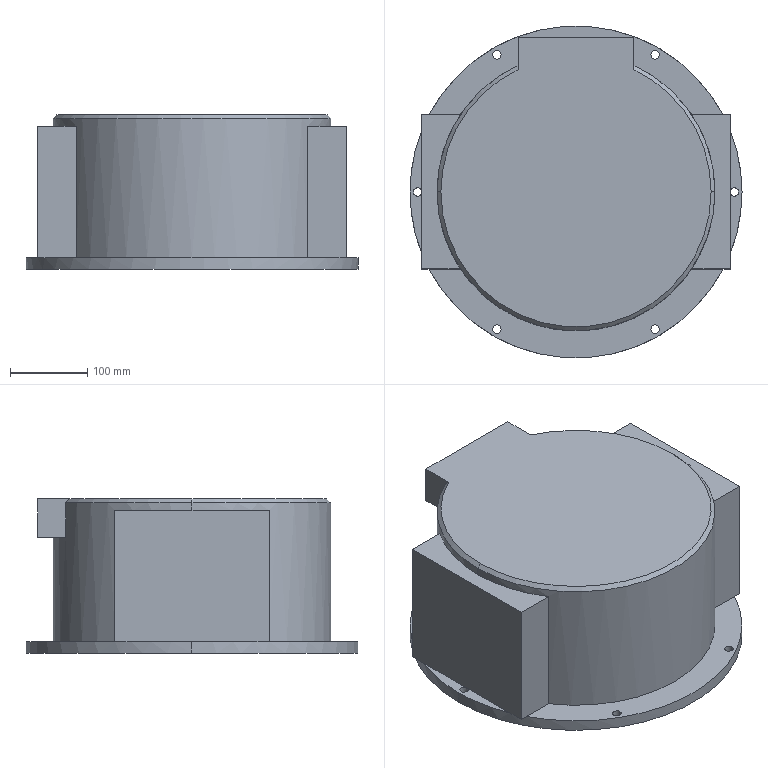Part | SolidWorks | features ICE 4, Chamfer 1, Extrusion 1, MirrorPattern 1 | 1 solid | 50 faces | box 430 x 430 x 200 mm | volume 23043977 mm3 | plane 29 | cylinder 18 | cone 3 | commonest cylinder face diameters 11 x12 50 x2 360 x2 430 x2
STEP:
#1=CARTESIAN_POINT('',(175.,0.,100.));
#2=VERTEX_POINT('',#1);
#3=CARTESIAN_POINT('',(75.,158.114,100.));
#4=VERTEX_POINT('',#3);
#5=CARTESIAN_POINT('',(0.,0.,100.));
#6=DIRECTION('',(0.,0.,1.));
#7=DIRECTION('',(1.,0.,0.));
#8=AXIS2_PLACEMENT_3D('',#5,#6,#7);
#9=CIRCLE('',#8,175.);
#10=EDGE_CURVE('',#2,#4,#9,.T.);
#11=ORIENTED_EDGE('',*,*,#10,.F.);
#12=CARTESIAN_POINT('',(180.,0.,95.));
#13=VERTEX_POINT('',#12);
#14=CARTESIAN_POINT('',(175.,0.,100.));
#15=DIRECTION('',(0.7071,0.,-0.7071));
#16=VECTOR('',#15,1000.);
#17=LINE('',#14,#16);
#18=EDGE_CURVE('',#2,#13,#17,.T.);
#19=ORIENTED_EDGE('',*,*,#18,.T.);
#20=CARTESIAN_POINT('',(75.,163.631,95.));
#21=VERTEX_POINT('',#20);
#22=CARTESIAN_POINT('',(0.,0.,95.));
#23=DIRECTION('',(0.,0.,-1.));
#24=DIRECTION('',(1.,0.,0.));
#25=AXIS2_PLACEMENT_3D('',#22,#23,#24);
#26=CIRCLE('',#25,180.);
#27=EDGE_CURVE('',#21,#13,#26,.T.);
#28=ORIENTED_EDGE('',*,*,#27,.F.);
#29=CARTESIAN_POINT('',(75.,158.114,100.));
#30=CARTESIAN_POINT('',(75.,159.955,98.336));
#31=CARTESIAN_POINT('',(75.,161.794,96.669));
#32=CARTESIAN_POINT('',(75.,163.631,95.));
#33=B_SPLINE_CURVE_WITH_KNOTS('',3,(#29,#30,#31,#32),.UNSPECIFIED.,.F.,.F.,(4,4),(0.,0.007445),.UNSPECIFIED.);
#34=EDGE_CURVE('',#4,#21,#33,.T.);
#35=ORIENTED_EDGE('',*,*,#34,.F.);
#36=EDGE_LOOP('',(#11,#19,#28,#35));
#37=FACE_OUTER_BOUND('',#36,.T.);
#38=CARTESIAN_POINT('',(0.,0.,100.));
#39=DIRECTION('',(0.,0.,-1.));
#40=DIRECTION('',(-1.,0.,0.));
#41=AXIS2_PLACEMENT_3D('',#38,#39,#40);
#42=CONICAL_SURFACE('',#41,175.,0.7854);
#43=ADVANCED_FACE('',(#37),#42,.T.);
#44=ORIENTED_EDGE('',*,*,#18,.F.);
#45=CARTESIAN_POINT('',(-175.,0.,100.));
#46=VERTEX_POINT('',#45);
#47=CARTESIAN_POINT('',(0.,0.,100.));
#48=DIRECTION('',(0.,0.,1.));
#49=DIRECTION('',(1.,0.,0.));
#50=AXIS2_PLACEMENT_3D('',#47,#48,#49);
#51=CIRCLE('',#50,175.);
#52=EDGE_CURVE('',#46,#2,#51,.T.);
#53=ORIENTED_EDGE('',*,*,#52,.F.);
#54=CARTESIAN_POINT('',(-180.,0.,95.));
#55=VERTEX_POINT('',#54);
#56=CARTESIAN_POINT('',(-175.,0.,100.));
#57=DIRECTION('',(-0.7071,0.,-0.7071));
#58=VECTOR('',#57,1000.);
#59=LINE('',#56,#58);
#60=EDGE_CURVE('',#46,#55,#59,.T.);
#61=ORIENTED_EDGE('',*,*,#60,.T.);
#62=CARTESIAN_POINT('',(0.,0.,95.));
#63=DIRECTION('',(0.,0.,-1.));
#64=DIRECTION('',(1.,0.,0.));
#65=AXIS2_PLACEMENT_3D('',#62,#63,#64);
#66=CIRCLE('',#65,180.);
#67=EDGE_CURVE('',#13,#55,#66,.T.);
#68=ORIENTED_EDGE('',*,*,#67,.F.);
#69=EDGE_LOOP('',(#44,#53,#61,#68));
#70=FACE_OUTER_BOUND('',#69,.T.);
#71=CARTESIAN_POINT('',(0.,0.,100.));
#72=DIRECTION('',(0.,0.,-1.));
#73=DIRECTION('',(-1.,0.,0.));
#74=AXIS2_PLACEMENT_3D('',#71,#72,#73);
#75=CONICAL_SURFACE('',#74,175.,0.7854);
#76=ADVANCED_FACE('',(#70),#75,.T.);
#77=CARTESIAN_POINT('',(25.,0.,-20.));
#78=VERTEX_POINT('',#77);
#79=CARTESIAN_POINT('',(-25.,0.,-20.));
#80=VERTEX_POINT('',#79);
#81=CARTESIAN_POINT('',(0.,0.,-20.));
#82=DIRECTION('',(0.,0.,-1.));
#83=DIRECTION('',(-1.,0.,0.));
#84=AXIS2_PLACEMENT_3D('',#81,#82,#83);
#85=CIRCLE('',#84,25.);
#86=EDGE_CURVE('',#78,#80,#85,.T.);
#87=ORIENTED_EDGE('',*,*,#86,.F.);
#88=CARTESIAN_POINT('',(25.,0.,-100.));
#89=VERTEX_POINT('',#88);
#90=CARTESIAN_POINT('',(25.,0.,-20.));
#91=DIRECTION('',(0.,0.,-1.));
#92=VECTOR('',#91,1000.);
#93=LINE('',#90,#92);
#94=EDGE_CURVE('',#78,#89,#93,.T.);
#95=ORIENTED_EDGE('',*,*,#94,.T.);
#96=CARTESIAN_POINT('',(-25.,0.,-100.));
#97=VERTEX_POINT('',#96);
#98=CARTESIAN_POINT('',(0.,0.,-100.));
#99=DIRECTION('',(0.,0.,-1.));
#100=DIRECTION('',(-1.,0.,0.));
#101=AXIS2_PLACEMENT_3D('',#98,#99,#100);
#102=CIRCLE('',#101,25.);
#103=EDGE_CURVE('',#89,#97,#102,.T.);
#104=ORIENTED_EDGE('',*,*,#103,.T.);
#105=CARTESIAN_POINT('',(-25.,0.,-20.));
#106=DIRECTION('',(0.,0.,-1.));
#107=VECTOR('',#106,1000.);
#108=LINE('',#105,#107);
#109=EDGE_CURVE('',#80,#97,#108,.T.);
#110=ORIENTED_EDGE('',*,*,#109,.F.);
#111=EDGE_LOOP('',(#87,#95,#104,#110));
#112=FACE_OUTER_BOUND('',#111,.T.);
#113=CARTESIAN_POINT('',(0.,0.,-20.));
#114=DIRECTION('',(0.,0.,-1.));
#115=DIRECTION('',(-1.,0.,0.));
#116=AXIS2_PLACEMENT_3D('',#113,#114,#115);
#117=CYLINDRICAL_SURFACE('',#116,25.);
#118=ADVANCED_FACE('',(#112),#117,.F.);
#119=CARTESIAN_POINT('',(210.5,0.,-85.));
#120=VERTEX_POINT('',#119);
#121=CARTESIAN_POINT('',(200.,-2.291,-85.));
#122=VERTEX_POINT('',#121);
#123=CARTESIAN_POINT('',(205.,0.,-85.));
#124=DIRECTION('',(0.,0.,-1.));
#125=DIRECTION('',(-1.,0.,0.));
#126=AXIS2_PLACEMENT_3D('',#123,#124,#125);
#127=CIRCLE('',#126,5.5);
#128=EDGE_CURVE('',#120,#122,#127,.T.);
#129=ORIENTED_EDGE('',*,*,#128,.F.);
#130=CARTESIAN_POINT('',(210.5,0.,-100.));
#131=VERTEX_POINT('',#130);
#132=CARTESIAN_POINT('',(210.5,0.,-85.));
#133=DIRECTION('',(0.,0.,-1.));
#134=VECTOR('',#133,1000.);
#135=LINE('',#132,#134);
#136=EDGE_CURVE('',#120,#131,#135,.T.);
#137=ORIENTED_EDGE('',*,*,#136,.T.);
#138=CARTESIAN_POINT('',(199.5,0.,-100.));
#139=VERTEX_POINT('',#138);
#140=CARTESIAN_POINT('',(205.,0.,-100.));
#141=DIRECTION('',(0.,0.,-1.));
#142=DIRECTION('',(-1.,0.,0.));
#143=AXIS2_PLACEMENT_3D('',#140,#141,#142);
#144=CIRCLE('',#143,5.5);
#145=EDGE_CURVE('',#131,#139,#144,.T.);
#146=ORIENTED_EDGE('',*,*,#145,.T.);
#147=CARTESIAN_POINT('',(199.5,0.,-85.));
#148=VERTEX_POINT('',#147);
#149=CARTESIAN_POINT('',(199.5,0.,-85.));
#150=DIRECTION('',(0.,0.,-1.));
#151=VECTOR('',#150,1000.);
#152=LINE('',#149,#151);
#153=EDGE_CURVE('',#148,#139,#152,.T.);
#154=ORIENTED_EDGE('',*,*,#153,.F.);
#155=CARTESIAN_POINT('',(205.,0.,-85.));
#156=DIRECTION('',(0.,0.,-1.));
#157=DIRECTION('',(-1.,0.,0.));
#158=AXIS2_PLACEMENT_3D('',#155,#156,#157);
#159=CIRCLE('',#158,5.5);
#160=EDGE_CURVE('',#122,#148,#159,.T.);
#161=ORIENTED_EDGE('',*,*,#160,.F.);
#162=EDGE_LOOP('',(#129,#137,#146,#154,#161));
#163=FACE_OUTER_BOUND('',#162,.T.);
#164=CARTESIAN_POINT('',(205.,0.,-85.));
#165=DIRECTION('',(0.,0.,-1.));
#166=DIRECTION('',(-1.,0.,0.));
#167=AXIS2_PLACEMENT_3D('',#164,#165,#166);
#168=CYLINDRICAL_SURFACE('',#167,5.5);
#169=ADVANCED_FACE('',(#163),#168,.F.);
#170=CARTESIAN_POINT('',(108.,-177.535,-85.));
#171=VERTEX_POINT('',#170);
#172=CARTESIAN_POINT('',(97.,-177.535,-85.));
#173=VERTEX_POINT('',#172);
#174=CARTESIAN_POINT('',(102.5,-177.535,-85.));
#175=DIRECTION('',(0.,0.,-1.));
#176=DIRECTION('',(-1.,0.,0.));
#177=AXIS2_PLACEMENT_3D('',#174,#175,#176);
#178=CIRCLE('',#177,5.5);
#179=EDGE_CURVE('',#171,#173,#178,.T.);
#180=ORIENTED_EDGE('',*,*,#179,.F.);
#181=CARTESIAN_POINT('',(108.,-177.535,-100.));
#182=VERTEX_POINT('',#181);
#183=CARTESIAN_POINT('',(108.,-177.535,-85.));
#184=DIRECTION('',(0.,0.,-1.));
#185=VECTOR('',#184,1000.);
#186=LINE('',#183,#185);
#187=EDGE_CURVE('',#171,#182,#186,.T.);
#188=ORIENTED_EDGE('',*,*,#187,.T.);
#189=CARTESIAN_POINT('',(97.,-177.535,-100.));
#190=VERTEX_POINT('',#189);
#191=CARTESIAN_POINT('',(102.5,-177.535,-100.));
#192=DIRECTION('',(0.,0.,-1.));
#193=DIRECTION('',(-1.,0.,0.));
#194=AXIS2_PLACEMENT_3D('',#191,#192,#193);
#195=CIRCLE('',#194,5.5);
#196=EDGE_CURVE('',#182,#190,#195,.T.);
#197=ORIENTED_EDGE('',*,*,#196,.T.);
#198=CARTESIAN_POINT('',(97.,-177.535,-85.));
#199=DIRECTION('',(0.,0.,-1.));
#200=VECTOR('',#199,1000.);
#201=LINE('',#198,#200);
#202=EDGE_CURVE('',#173,#190,#201,.T.);
#203=ORIENTED_EDGE('',*,*,#202,.F.);
#204=EDGE_LOOP('',(#180,#188,#197,#203));
#205=FACE_OUTER_BOUND('',#204,.T.);
#206=CARTESIAN_POINT('',(102.5,-177.535,-85.));
#207=DIRECTION('',(0.,0.,-1.));
#208=DIRECTION('',(-1.,0.,0.));
#209=AXIS2_PLACEMENT_3D('',#206,#207,#208);
#210=CYLINDRICAL_SURFACE('',#209,5.5);
#211=ADVANCED_FACE('',(#205),#210,.F.);
#212=CARTESIAN_POINT('',(-97.,-177.535,-85.));
#213=VERTEX_POINT('',#212);
#214=CARTESIAN_POINT('',(-108.,-177.535,-85.));
#215=VERTEX_POINT('',#214);
#216=CARTESIAN_POINT('',(-102.5,-177.535,-85.));
#217=DIRECTION('',(0.,0.,-1.));
#218=DIRECTION('',(-1.,0.,0.));
#219=AXIS2_PLACEMENT_3D('',#216,#217,#218);
#220=CIRCLE('',#219,5.5);
#221=EDGE_CURVE('',#213,#215,#220,.T.);
#222=ORIENTED_EDGE('',*,*,#221,.F.);
#223=CARTESIAN_POINT('',(-97.,-177.535,-100.));
#224=VERTEX_POINT('',#223);
#225=CARTESIAN_POINT('',(-97.,-177.535,-85.));
#226=DIRECTION('',(0.,0.,-1.));
#227=VECTOR('',#226,1000.);
#228=LINE('',#225,#227);
#229=EDGE_CURVE('',#213,#224,#228,.T.);
#230=ORIENTED_EDGE('',*,*,#229,.T.);
#231=CARTESIAN_POINT('',(-108.,-177.535,-100.));
#232=VERTEX_POINT('',#231);
#233=CARTESIAN_POINT('',(-102.5,-177.535,-100.));
#234=DIRECTION('',(0.,0.,-1.));
#235=DIRECTION('',(-1.,0.,0.));
#236=AXIS2_PLACEMENT_3D('',#233,#234,#235);
#237=CIRCLE('',#236,5.5);
#238=EDGE_CURVE('',#224,#232,#237,.T.);
#239=ORIENTED_EDGE('',*,*,#238,.T.);
#240=CARTESIAN_POINT('',(-108.,-177.535,-85.));
#241=DIRECTION('',(0.,0.,-1.));
#242=VECTOR('',#241,1000.);
#243=LINE('',#240,#242);
#244=EDGE_CURVE('',#215,#232,#243,.T.);
#245=ORIENTED_EDGE('',*,*,#244,.F.);
#246=EDGE_LOOP('',(#222,#230,#239,#245));
#247=FACE_OUTER_BOUND('',#246,.T.);
#248=CARTESIAN_POINT('',(-102.5,-177.535,-85.));
#249=DIRECTION('',(0.,0.,-1.));
#250=DIRECTION('',(-1.,0.,0.));
#251=AXIS2_PLACEMENT_3D('',#248,#249,#250);
#252=CYLINDRICAL_SURFACE('',#251,5.5);
#253=ADVANCED_FACE('',(#247),#252,.F.);
#254=CARTESIAN_POINT('',(-199.5,0.,-85.));
#255=VERTEX_POINT('',#254);
#256=CARTESIAN_POINT('',(-200.,-2.291,-85.));
#257=VERTEX_POINT('',#256);
#258=CARTESIAN_POINT('',(-205.,0.,-85.));
#259=DIRECTION('',(0.,0.,-1.));
#260=DIRECTION('',(-1.,0.,0.));
#261=AXIS2_PLACEMENT_3D('',#258,#259,#260);
#262=CIRCLE('',#261,5.5);
#263=EDGE_CURVE('',#255,#257,#262,.T.);
#264=ORIENTED_EDGE('',*,*,#263,.F.);
#265=CARTESIAN_POINT('',(-199.5,0.,-100.));
#266=VERTEX_POINT('',#265);
#267=CARTESIAN_POINT('',(-199.5,0.,-85.));
#268=DIRECTION('',(0.,0.,-1.));
#269=VECTOR('',#268,1000.);
#270=LINE('',#267,#269);
#271=EDGE_CURVE('',#255,#266,#270,.T.);
#272=ORIENTED_EDGE('',*,*,#271,.T.);
#273=CARTESIAN_POINT('',(-210.5,0.,-100.));
#274=VERTEX_POINT('',#273);
#275=CARTESIAN_POINT('',(-205.,0.,-100.));
#276=DIRECTION('',(0.,0.,-1.));
#277=DIRECTION('',(-1.,0.,0.));
#278=AXIS2_PLACEMENT_3D('',#275,#276,#277);
#279=CIRCLE('',#278,5.5);
#280=EDGE_CURVE('',#266,#274,#279,.T.);
#281=ORIENTED_EDGE('',*,*,#280,.T.);
#282=CARTESIAN_POINT('',(-210.5,0.,-85.));
#283=VERTEX_POINT('',#282);
#284=CARTESIAN_POINT('',(-210.5,0.,-85.));
#285=DIRECTION('',(0.,0.,-1.));
#286=VECTOR('',#285,1000.);
#287=LINE('',#284,#286);
#288=EDGE_CURVE('',#283,#274,#287,.T.);
#289=ORIENTED_EDGE('',*,*,#288,.F.);
#290=CARTESIAN_POINT('',(-205.,0.,-85.));
#291=DIRECTION('',(0.,0.,-1.));
#292=DIRECTION('',(-1.,0.,0.));
#293=AXIS2_PLACEMENT_3D('',#290,#291,#292);
#294=CIRCLE('',#293,5.5);
#295=EDGE_CURVE('',#257,#283,#294,.T.);
#296=ORIENTED_EDGE('',*,*,#295,.F.);
#297=EDGE_LOOP('',(#264,#272,#281,#289,#296));
#298=FACE_OUTER_BOUND('',#297,.T.);
#299=CARTESIAN_POINT('',(-205.,0.,-85.));
#300=DIRECTION('',(0.,0.,-1.));
#301=DIRECTION('',(-1.,0.,0.));
#302=AXIS2_PLACEMENT_3D('',#299,#300,#301);
#303=CYLINDRICAL_SURFACE('',#302,5.5);
#304=ADVANCED_FACE('',(#298),#303,.F.);
#305=CARTESIAN_POINT('',(-97.,177.535,-85.));
#306=VERTEX_POINT('',#305);
#307=CARTESIAN_POINT('',(-108.,177.535,-85.));
#308=VERTEX_POINT('',#307);
#309=CARTESIAN_POINT('',(-102.5,177.535,-85.));
#310=DIRECTION('',(0.,0.,-1.));
#311=DIRECTION('',(-1.,0.,0.));
#312=AXIS2_PLACEMENT_3D('',#309,#310,#311);
#313=CIRCLE('',#312,5.5);
#314=EDGE_CURVE('',#306,#308,#313,.T.);
#315=ORIENTED_EDGE('',*,*,#314,.F.);
#316=CARTESIAN_POINT('',(-97.,177.535,-100.));
#317=VERTEX_POINT('',#316);
#318=CARTESIAN_POINT('',(-97.,177.535,-85.));
#319=DIRECTION('',(0.,0.,-1.));
#320=VECTOR('',#319,1000.);
#321=LINE('',#318,#320);
#322=EDGE_CURVE('',#306,#317,#321,.T.);
#323=ORIENTED_EDGE('',*,*,#322,.T.);
#324=CARTESIAN_POINT('',(-108.,177.535,-100.));
#325=VERTEX_POINT('',#324);
#326=CARTESIAN_POINT('',(-102.5,177.535,-100.));
#327=DIRECTION('',(0.,0.,-1.));
#328=DIRECTION('',(-1.,0.,0.));
#329=AXIS2_PLACEMENT_3D('',#326,#327,#328);
#330=CIRCLE('',#329,5.5);
#331=EDGE_CURVE('',#317,#325,#330,.T.);
#332=ORIENTED_EDGE('',*,*,#331,.T.);
#333=CARTESIAN_POINT('',(-108.,177.535,-85.));
#334=DIRECTION('',(0.,0.,-1.));
#335=VECTOR('',#334,1000.);
#336=LINE('',#333,#335);
#337=EDGE_CURVE('',#308,#325,#336,.T.);
#338=ORIENTED_EDGE('',*,*,#337,.F.);
#339=EDGE_LOOP('',(#315,#323,#332,#338));
#340=FACE_OUTER_BOUND('',#339,.T.);
#341=CARTESIAN_POINT('',(-102.5,177.535,-85.));
#342=DIRECTION('',(0.,0.,-1.));
#343=DIRECTION('',(-1.,0.,0.));
#344=AXIS2_PLACEMENT_3D('',#341,#342,#343);
#345=CYLINDRICAL_SURFACE('',#344,5.5);
#346=ADVANCED_FACE('',(#340),#345,.F.);
#347=CARTESIAN_POINT('',(108.,177.535,-85.));
#348=VERTEX_POINT('',#347);
#349=CARTESIAN_POINT('',(97.,177.535,-85.));
#350=VERTEX_POINT('',#349);
#351=CARTESIAN_POINT('',(102.5,177.535,-85.));
#352=DIRECTION('',(0.,0.,-1.));
#353=DIRECTION('',(-1.,0.,0.));
#354=AXIS2_PLACEMENT_3D('',#351,#352,#353);
#355=CIRCLE('',#354,5.5);
#356=EDGE_CURVE('',#348,#350,#355,.T.);
#357=ORIENTED_EDGE('',*,*,#356,.F.);
#358=CARTESIAN_POINT('',(108.,177.535,-100.));
#359=VERTEX_POINT('',#358);
#360=CARTESIAN_POINT('',(108.,177.535,-85.));
#361=DIRECTION('',(0.,0.,-1.));
#362=VECTOR('',#361,1000.);
#363=LINE('',#360,#362);
#364=EDGE_CURVE('',#348,#359,#363,.T.);
#365=ORIENTED_EDGE('',*,*,#364,.T.);
#366=CARTESIAN_POINT('',(97.,177.535,-100.));
#367=VERTEX_POINT('',#366);
#368=CARTESIAN_POINT('',(102.5,177.535,-100.));
#369=DIRECTION('',(0.,0.,-1.));
#370=DIRECTION('',(-1.,0.,0.));
#371=AXIS2_PLACEMENT_3D('',#368,#369,#370);
#372=CIRCLE('',#371,5.5);
#373=EDGE_CURVE('',#359,#367,#372,.T.);
#374=ORIENTED_EDGE('',*,*,#373,.T.);
#375=CARTESIAN_POINT('',(97.,177.535,-85.));
#376=DIRECTION('',(0.,0.,-1.));
#377=VECTOR('',#376,1000.);
#378=LINE('',#375,#377);
#379=EDGE_CURVE('',#350,#367,#378,.T.);
#380=ORIENTED_EDGE('',*,*,#379,.F.);
#381=EDGE_LOOP('',(#357,#365,#374,#380));
#382=FACE_OUTER_BOUND('',#381,.T.);
#383=CARTESIAN_POINT('',(102.5,177.535,-85.));
#384=DIRECTION('',(0.,0.,-1.));
#385=DIRECTION('',(-1.,0.,0.));
#386=AXIS2_PLACEMENT_3D('',#383,#384,#385);
#387=CYLINDRICAL_SURFACE('',#386,5.5);
#388=ADVANCED_FACE('',(#382),#387,.F.);
#389=CARTESIAN_POINT('',(200.,78.899,-85.));
#390=VERTEX_POINT('',#389);
#391=CARTESIAN_POINT('',(215.,0.,-85.));
#392=VERTEX_POINT('',#391);
#393=CARTESIAN_POINT('',(0.,0.,-85.));
#394=DIRECTION('',(0.,0.,-1.));
#395=DIRECTION('',(-1.,0.,0.));
#396=AXIS2_PLACEMENT_3D('',#393,#394,#395);
#397=CIRCLE('',#396,215.);
#398=EDGE_CURVE('',#390,#392,#397,.T.);
#399=ORIENTED_EDGE('',*,*,#398,.T.);
#400=CARTESIAN_POINT('',(215.,0.,-100.));
#401=VERTEX_POINT('',#400);
#402=CARTESIAN_POINT('',(215.,0.,-85.));
#403=DIRECTION('',(0.,0.,-1.));
#404=VECTOR('',#403,1000.);
#405=LINE('',#402,#404);
#406=EDGE_CURVE('',#392,#401,#405,.T.);
#407=ORIENTED_EDGE('',*,*,#406,.T.);
#408=CARTESIAN_POINT('',(-215.,0.,-100.));
#409=VERTEX_POINT('',#408);
#410=CARTESIAN_POINT('',(0.,0.,-100.));
#411=DIRECTION('',(0.,0.,-1.));
#412=DIRECTION('',(-1.,0.,0.));
#413=AXIS2_PLACEMENT_3D('',#410,#411,#412);
#414=CIRCLE('',#413,215.);
#415=EDGE_CURVE('',#409,#401,#414,.T.);
#416=ORIENTED_EDGE('',*,*,#415,.F.);
#417=CARTESIAN_POINT('',(-215.,0.,-85.));
#418=VERTEX_POINT('',#417);
#419=CARTESIAN_POINT('',(-215.,0.,-85.));
#420=DIRECTION('',(0.,0.,-1.));
#421=VECTOR('',#420,1000.);
#422=LINE('',#419,#421);
#423=EDGE_CURVE('',#418,#409,#422,.T.);
#424=ORIENTED_EDGE('',*,*,#423,.F.);
#425=CARTESIAN_POINT('',(-200.,78.899,-85.));
#426=VERTEX_POINT('',#425);
#427=CARTESIAN_POINT('',(0.,0.,-85.));
#428=DIRECTION('',(0.,0.,-1.));
#429=DIRECTION('',(-1.,0.,0.));
#430=AXIS2_PLACEMENT_3D('',#427,#428,#429);
#431=CIRCLE('',#430,215.);
#432=EDGE_CURVE('',#418,#426,#431,.T.);
#433=ORIENTED_EDGE('',*,*,#432,.T.);
#434=CARTESIAN_POINT('',(-190.329,100.,-85.));
#435=VERTEX_POINT('',#434);
#436=CARTESIAN_POINT('',(0.,0.,-85.));
#437=DIRECTION('',(0.,0.,1.));
#438=DIRECTION('',(-1.,0.,0.));
#439=AXIS2_PLACEMENT_3D('',#436,#437,#438);
#440=CIRCLE('',#439,215.);
#441=EDGE_CURVE('',#435,#426,#440,.T.);
#442=ORIENTED_EDGE('',*,*,#441,.F.);
#443=CARTESIAN_POINT('',(190.329,100.,-85.));
#444=VERTEX_POINT('',#443);
#445=CARTESIAN_POINT('',(0.,0.,-85.));
#446=DIRECTION('',(0.,0.,-1.));
#447=DIRECTION('',(-1.,0.,0.));
#448=AXIS2_PLACEMENT_3D('',#445,#446,#447);
#449=CIRCLE('',#448,215.);
#450=EDGE_CURVE('',#435,#444,#449,.T.);
#451=ORIENTED_EDGE('',*,*,#450,.T.);
#452=CARTESIAN_POINT('',(0.,0.,-85.));
#453=DIRECTION('',(0.,0.,-1.));
#454=DIRECTION('',(-1.,0.,0.));
#455=AXIS2_PLACEMENT_3D('',#452,#453,#454);
#456=CIRCLE('',#455,215.);
#457=EDGE_CURVE('',#444,#390,#456,.T.);
#458=ORIENTED_EDGE('',*,*,#457,.T.);
#459=EDGE_LOOP('',(#399,#407,#416,#424,#433,#442,#451,#458));
#460=FACE_OUTER_BOUND('',#459,.T.);
#461=CARTESIAN_POINT('',(0.,0.,-85.));
#462=DIRECTION('',(0.,0.,-1.));
#463=DIRECTION('',(-1.,0.,0.));
#464=AXIS2_PLACEMENT_3D('',#461,#462,#463);
#465=CYLINDRICAL_SURFACE('',#464,215.);
#466=ADVANCED_FACE('',(#460),#465,.T.);
#467=ORIENTED_EDGE('',*,*,#27,.T.);
#468=CARTESIAN_POINT('',(180.,0.,85.));
#469=VERTEX_POINT('',#468);
#470=CARTESIAN_POINT('',(180.,0.,100.));
#471=DIRECTION('',(0.,0.,-1.));
#472=VECTOR('',#471,1000.);
#473=LINE('',#470,#472);
#474=EDGE_CURVE('',#13,#469,#473,.T.);
#475=ORIENTED_EDGE('',*,*,#474,.T.);
#476=CARTESIAN_POINT('',(150.,99.499,85.));
#477=VERTEX_POINT('',#476);
#478=CARTESIAN_POINT('',(0.,0.,85.));
#479=DIRECTION('',(0.,0.,-1.));
#480=DIRECTION('',(-1.,0.,0.));
#481=AXIS2_PLACEMENT_3D('',#478,#479,#480);
#482=CIRCLE('',#481,180.);
#483=EDGE_CURVE('',#477,#469,#482,.T.);
#484=ORIENTED_EDGE('',*,*,#483,.F.);
#485=CARTESIAN_POINT('',(150.,99.499,-85.));
#486=VERTEX_POINT('',#485);
#487=CARTESIAN_POINT('',(150.,99.499,100.));
#488=DIRECTION('',(0.,0.,1.));
#489=VECTOR('',#488,1000.);
#490=LINE('',#487,#489);
#491=EDGE_CURVE('',#486,#477,#490,.T.);
#492=ORIENTED_EDGE('',*,*,#491,.F.);
#493=CARTESIAN_POINT('',(-150.,99.499,-85.));
#494=VERTEX_POINT('',#493);
#495=CARTESIAN_POINT('',(0.,0.,-85.));
#496=DIRECTION('',(0.,0.,-1.));
#497=DIRECTION('',(-1.,0.,0.));
#498=AXIS2_PLACEMENT_3D('',#495,#496,#497);
#499=CIRCLE('',#498,180.);
#500=EDGE_CURVE('',#494,#486,#499,.T.);
#501=ORIENTED_EDGE('',*,*,#500,.F.);
#502=CARTESIAN_POINT('',(-150.,99.499,85.));
#503=VERTEX_POINT('',#502);
#504=CARTESIAN_POINT('',(-150.,99.499,100.));
#505=DIRECTION('',(0.,0.,-1.));
#506=VECTOR('',#505,1000.);
#507=LINE('',#504,#506);
#508=EDGE_CURVE('',#503,#494,#507,.T.);
#509=ORIENTED_EDGE('',*,*,#508,.F.);
#510=CARTESIAN_POINT('',(-180.,0.,85.));
#511=VERTEX_POINT('',#510);
#512=CARTESIAN_POINT('',(0.,0.,85.));
#513=DIRECTION('',(0.,0.,1.));
#514=DIRECTION('',(1.,0.,0.));
#515=AXIS2_PLACEMENT_3D('',#512,#513,#514);
#516=CIRCLE('',#515,180.);
#517=EDGE_CURVE('',#503,#511,#516,.T.);
#518=ORIENTED_EDGE('',*,*,#517,.T.);
#519=CARTESIAN_POINT('',(-180.,0.,100.));
#520=DIRECTION('',(0.,0.,-1.));
#521=VECTOR('',#520,1000.);
#522=LINE('',#519,#521);
#523=EDGE_CURVE('',#55,#511,#522,.T.);
#524=ORIENTED_EDGE('',*,*,#523,.F.);
#525=CARTESIAN_POINT('',(-75.,163.631,95.));
#526=VERTEX_POINT('',#525);
#527=CARTESIAN_POINT('',(0.,0.,95.));
#528=DIRECTION('',(0.,0.,-1.));
#529=DIRECTION('',(1.,0.,0.));
#530=AXIS2_PLACEMENT_3D('',#527,#528,#529);
#531=CIRCLE('',#530,180.);
#532=EDGE_CURVE('',#55,#526,#531,.T.);
#533=ORIENTED_EDGE('',*,*,#532,.T.);
#534=CARTESIAN_POINT('',(-75.,163.631,50.));
#535=VERTEX_POINT('',#534);
#536=CARTESIAN_POINT('',(-75.,163.631,100.));
#537=DIRECTION('',(0.,0.,-1.));
#538=VECTOR('',#537,1000.);
#539=LINE('',#536,#538);
#540=EDGE_CURVE('',#526,#535,#539,.T.);
#541=ORIENTED_EDGE('',*,*,#540,.T.);
#542=CARTESIAN_POINT('',(75.,163.631,50.));
#543=VERTEX_POINT('',#542);
#544=CARTESIAN_POINT('',(0.,0.,50.));
#545=DIRECTION('',(0.,0.,1.));
#546=DIRECTION('',(1.,0.,0.));
#547=AXIS2_PLACEMENT_3D('',#544,#545,#546);
#548=CIRCLE('',#547,180.);
#549=EDGE_CURVE('',#543,#535,#548,.T.);
#550=ORIENTED_EDGE('',*,*,#549,.F.);
#551=CARTESIAN_POINT('',(75.,163.631,100.));
#552=DIRECTION('',(0.,0.,1.));
#553=VECTOR('',#552,1000.);
#554=LINE('',#551,#553);
#555=EDGE_CURVE('',#543,#21,#554,.T.);
#556=ORIENTED_EDGE('',*,*,#555,.T.);
#557=EDGE_LOOP('',(#467,#475,#484,#492,#501,#509,#518,#524,#533,#541,#550,#556));
#558=FACE_OUTER_BOUND('',#557,.T.);
#559=CARTESIAN_POINT('',(0.,0.,100.));
#560=DIRECTION('',(0.,0.,-1.));
#561=DIRECTION('',(-1.,0.,0.));
#562=AXIS2_PLACEMENT_3D('',#559,#560,#561);
#563=CYLINDRICAL_SURFACE('',#562,180.);
#564=ADVANCED_FACE('',(#558),#563,.T.);
#565=ORIENTED_EDGE('',*,*,#474,.F.);
#566=ORIENTED_EDGE('',*,*,#67,.T.);
#567=ORIENTED_EDGE('',*,*,#523,.T.);
#568=CARTESIAN_POINT('',(-150.,-99.499,85.));
#569=VERTEX_POINT('',#568);
#570=CARTESIAN_POINT('',(0.,0.,85.));
#571=DIRECTION('',(0.,0.,1.));
#572=DIRECTION('',(1.,0.,0.));
#573=AXIS2_PLACEMENT_3D('',#570,#571,#572);
#574=CIRCLE('',#573,180.);
#575=EDGE_CURVE('',#511,#569,#574,.T.);
#576=ORIENTED_EDGE('',*,*,#575,.T.);
#577=CARTESIAN_POINT('',(-150.,-99.499,-85.));
#578=VERTEX_POINT('',#577);
#579=CARTESIAN_POINT('',(-150.,-99.499,100.));
#580=DIRECTION('',(0.,0.,1.));
#581=VECTOR('',#580,1000.);
#582=LINE('',#579,#581);
#583=EDGE_CURVE('',#578,#569,#582,.T.);
#584=ORIENTED_EDGE('',*,*,#583,.F.);
#585=CARTESIAN_POINT('',(150.,-99.499,-85.));
#586=VERTEX_POINT('',#585);
#587=CARTESIAN_POINT('',(0.,0.,-85.));
#588=DIRECTION('',(0.,0.,-1.));
#589=DIRECTION('',(-1.,0.,0.));
#590=AXIS2_PLACEMENT_3D('',#587,#588,#589);
#591=CIRCLE('',#590,180.);
#592=EDGE_CURVE('',#586,#578,#591,.T.);
#593=ORIENTED_EDGE('',*,*,#592,.F.);
#594=CARTESIAN_POINT('',(150.,-99.499,85.));
#595=VERTEX_POINT('',#594);
#596=CARTESIAN_POINT('',(150.,-99.499,100.));
#597=DIRECTION('',(0.,0.,-1.));
#598=VECTOR('',#597,1000.);
#599=LINE('',#596,#598);
#600=EDGE_CURVE('',#595,#586,#599,.T.);
#601=ORIENTED_EDGE('',*,*,#600,.F.);
#602=CARTESIAN_POINT('',(0.,0.,85.));
#603=DIRECTION('',(0.,0.,-1.));
#604=DIRECTION('',(-1.,0.,0.));
#605=AXIS2_PLACEMENT_3D('',#602,#603,#604);
#606=CIRCLE('',#605,180.);
#607=EDGE_CURVE('',#469,#595,#606,.T.);
#608=ORIENTED_EDGE('',*,*,#607,.F.);
#609=EDGE_LOOP('',(#565,#566,#567,#576,#584,#593,#601,#608));
#610=FACE_OUTER_BOUND('',#609,.T.);
#611=CARTESIAN_POINT('',(0.,0.,100.));
#612=DIRECTION('',(0.,0.,-1.));
#613=DIRECTION('',(-1.,0.,0.));
#614=AXIS2_PLACEMENT_3D('',#611,#612,#613);
#615=CYLINDRICAL_SURFACE('',#614,180.);
#616=ADVANCED_FACE('',(#610),#615,.T.);
#617=CARTESIAN_POINT('',(-200.,-78.899,-85.));
#618=VERTEX_POINT('',#617);
#619=CARTESIAN_POINT('',(0.,0.,-85.));
#620=DIRECTION('',(0.,0.,-1.));
#621=DIRECTION('',(-1.,0.,0.));
#622=AXIS2_PLACEMENT_3D('',#619,#620,#621);
#623=CIRCLE('',#622,215.);
#624=EDGE_CURVE('',#618,#418,#623,.T.);
#625=ORIENTED_EDGE('',*,*,#624,.F.);
#626=CARTESIAN_POINT('',(-200.,100.,-85.));
#627=DIRECTION('',(0.,1.,0.));
#628=VECTOR('',#627,1000.);
#629=LINE('',#626,#628);
#630=EDGE_CURVE('',#618,#257,#629,.T.);
#631=ORIENTED_EDGE('',*,*,#630,.T.);
#632=ORIENTED_EDGE('',*,*,#295,.T.);
#633=CARTESIAN_POINT('',(-200.,2.291,-85.));
#634=VERTEX_POINT('',#633);
#635=CARTESIAN_POINT('',(-205.,0.,-85.));
#636=DIRECTION('',(0.,0.,-1.));
#637=DIRECTION('',(-1.,0.,0.));
#638=AXIS2_PLACEMENT_3D('',#635,#636,#637);
#639=CIRCLE('',#638,5.5);
#640=EDGE_CURVE('',#283,#634,#639,.T.);
#641=ORIENTED_EDGE('',*,*,#640,.T.);
#642=CARTESIAN_POINT('',(-200.,100.,-85.));
#643=DIRECTION('',(0.,1.,0.));
#644=VECTOR('',#643,1000.);
#645=LINE('',#642,#644);
#646=EDGE_CURVE('',#634,#426,#645,.T.);
#647=ORIENTED_EDGE('',*,*,#646,.T.);
#648=ORIENTED_EDGE('',*,*,#432,.F.);
#649=EDGE_LOOP('',(#625,#631,#632,#641,#647,#648));
#650=FACE_OUTER_BOUND('',#649,.T.);
#651=CARTESIAN_POINT('',(0.,0.,-85.));
#652=DIRECTION('',(0.,0.,-1.));
#653=DIRECTION('',(-1.,0.,0.));
#654=AXIS2_PLACEMENT_3D('',#651,#652,#653);
#655=PLANE('',#654);
#656=ADVANCED_FACE('',(#650),#655,.F.);
#657=CARTESIAN_POINT('',(102.5,-177.535,-85.));
#658=DIRECTION('',(0.,0.,-1.));
#659=DIRECTION('',(-1.,0.,0.));
#660=AXIS2_PLACEMENT_3D('',#657,#658,#659);
#661=CIRCLE('',#660,5.5);
#662=EDGE_CURVE('',#173,#171,#661,.T.);
#663=ORIENTED_EDGE('',*,*,#662,.T.);
#664=ORIENTED_EDGE('',*,*,#179,.T.);
#665=EDGE_LOOP('',(#663,#664));
#666=FACE_BOUND('',#665,.T.);
#667=CARTESIAN_POINT('',(-102.5,-177.535,-85.));
#668=DIRECTION('',(0.,0.,-1.));
#669=DIRECTION('',(-1.,0.,0.));
#670=AXIS2_PLACEMENT_3D('',#667,#668,#669);
#671=CIRCLE('',#670,5.5);
#672=EDGE_CURVE('',#215,#213,#671,.T.);
#673=ORIENTED_EDGE('',*,*,#672,.T.);
#674=ORIENTED_EDGE('',*,*,#221,.T.);
#675=EDGE_LOOP('',(#673,#674));
#676=FACE_BOUND('',#675,.T.);
#677=CARTESIAN_POINT('',(-150.,-100.,-85.));
#678=VERTEX_POINT('',#677);
#679=CARTESIAN_POINT('',(-150.,100.,-85.));
#680=DIRECTION('',(0.,1.,0.));
#681=VECTOR('',#680,1000.);
#682=LINE('',#679,#681);
#683=EDGE_CURVE('',#678,#578,#682,.T.);
#684=ORIENTED_EDGE('',*,*,#683,.F.);
#685=CARTESIAN_POINT('',(-190.329,-100.,-85.));
#686=VERTEX_POINT('',#685);
#687=CARTESIAN_POINT('',(-200.,-100.,-85.));
#688=DIRECTION('',(1.,0.,0.));
#689=VECTOR('',#688,1000.);
#690=LINE('',#687,#689);
#691=EDGE_CURVE('',#686,#678,#690,.T.);
#692=ORIENTED_EDGE('',*,*,#691,.F.);
#693=CARTESIAN_POINT('',(190.329,-100.,-85.));
#694=VERTEX_POINT('',#693);
#695=CARTESIAN_POINT('',(0.,0.,-85.));
#696=DIRECTION('',(0.,0.,-1.));
#697=DIRECTION('',(-1.,0.,0.));
#698=AXIS2_PLACEMENT_3D('',#695,#696,#697);
#699=CIRCLE('',#698,215.);
#700=EDGE_CURVE('',#694,#686,#699,.T.);
#701=ORIENTED_EDGE('',*,*,#700,.F.);
#702=CARTESIAN_POINT('',(150.,-100.,-85.));
#703=VERTEX_POINT('',#702);
#704=CARTESIAN_POINT('',(200.,-100.,-85.));
#705=DIRECTION('',(-1.,0.,0.));
#706=VECTOR('',#705,1000.);
#707=LINE('',#704,#706);
#708=EDGE_CURVE('',#694,#703,#707,.T.);
#709=ORIENTED_EDGE('',*,*,#708,.T.);
#710=CARTESIAN_POINT('',(150.,100.,-85.));
#711=DIRECTION('',(0.,1.,0.));
#712=VECTOR('',#711,1000.);
#713=LINE('',#710,#712);
#714=EDGE_CURVE('',#703,#586,#713,.T.);
#715=ORIENTED_EDGE('',*,*,#714,.T.);
#716=ORIENTED_EDGE('',*,*,#592,.T.);
#717=EDGE_LOOP('',(#684,#692,#701,#709,#715,#716));
#718=FACE_OUTER_BOUND('',#717,.T.);
#719=CARTESIAN_POINT('',(0.,0.,-85.));
#720=DIRECTION('',(0.,0.,-1.));
#721=DIRECTION('',(-1.,0.,0.));
#722=AXIS2_PLACEMENT_3D('',#719,#720,#721);
#723=PLANE('',#722);
#724=ADVANCED_FACE('',(#666,#676,#718),#723,.F.);
#725=CARTESIAN_POINT('',(102.5,177.535,-85.));
#726=DIRECTION('',(0.,0.,-1.));
#727=DIRECTION('',(-1.,0.,0.));
#728=AXIS2_PLACEMENT_3D('',#725,#726,#727);
#729=CIRCLE('',#728,5.5);
#730=EDGE_CURVE('',#350,#348,#729,.T.);
#731=ORIENTED_EDGE('',*,*,#730,.T.);
#732=ORIENTED_EDGE('',*,*,#356,.T.);
#733=EDGE_LOOP('',(#731,#732));
#734=FACE_BOUND('',#733,.T.);
#735=CARTESIAN_POINT('',(-102.5,177.535,-85.));
#736=DIRECTION('',(0.,0.,-1.));
#737=DIRECTION('',(-1.,0.,0.));
#738=AXIS2_PLACEMENT_3D('',#735,#736,#737);
#739=CIRCLE('',#738,5.5);
#740=EDGE_CURVE('',#308,#306,#739,.T.);
#741=ORIENTED_EDGE('',*,*,#740,.T.);
#742=ORIENTED_EDGE('',*,*,#314,.T.);
#743=EDGE_LOOP('',(#741,#742));
#744=FACE_BOUND('',#743,.T.);
#745=ORIENTED_EDGE('',*,*,#450,.F.);
#746=CARTESIAN_POINT('',(-150.,100.,-85.));
#747=VERTEX_POINT('',#746);
#748=CARTESIAN_POINT('',(-200.,100.,-85.));
#749=DIRECTION('',(1.,0.,0.));
#750=VECTOR('',#749,1000.);
#751=LINE('',#748,#750);
#752=EDGE_CURVE('',#435,#747,#751,.T.);
#753=ORIENTED_EDGE('',*,*,#752,.T.);
#754=CARTESIAN_POINT('',(-150.,100.,-85.));
#755=DIRECTION('',(0.,1.,0.));
#756=VECTOR('',#755,1000.);
#757=LINE('',#754,#756);
#758=EDGE_CURVE('',#494,#747,#757,.T.);
#759=ORIENTED_EDGE('',*,*,#758,.F.);
#760=ORIENTED_EDGE('',*,*,#500,.T.);
#761=CARTESIAN_POINT('',(150.,100.,-85.));
#762=VERTEX_POINT('',#761);
#763=CARTESIAN_POINT('',(150.,100.,-85.));
#764=DIRECTION('',(0.,1.,0.));
#765=VECTOR('',#764,1000.);
#766=LINE('',#763,#765);
#767=EDGE_CURVE('',#486,#762,#766,.T.);
#768=ORIENTED_EDGE('',*,*,#767,.T.);
#769=CARTESIAN_POINT('',(200.,100.,-85.));
#770=DIRECTION('',(-1.,0.,0.));
#771=VECTOR('',#770,1000.);
#772=LINE('',#769,#771);
#773=EDGE_CURVE('',#444,#762,#772,.T.);
#774=ORIENTED_EDGE('',*,*,#773,.F.);
#775=EDGE_LOOP('',(#745,#753,#759,#760,#768,#774));
#776=FACE_OUTER_BOUND('',#775,.T.);
#777=CARTESIAN_POINT('',(0.,0.,-85.));
#778=DIRECTION('',(0.,0.,-1.));
#779=DIRECTION('',(-1.,0.,0.));
#780=AXIS2_PLACEMENT_3D('',#777,#778,#779);
#781=PLANE('',#780);
#782=ADVANCED_FACE('',(#734,#744,#776),#781,.F.);
#783=CARTESIAN_POINT('',(-75.,158.114,100.));
#784=VERTEX_POINT('',#783);
#785=CARTESIAN_POINT('',(0.,0.,100.));
#786=DIRECTION('',(0.,0.,1.));
#787=DIRECTION('',(1.,0.,0.));
#788=AXIS2_PLACEMENT_3D('',#785,#786,#787);
#789=CIRCLE('',#788,175.);
#790=EDGE_CURVE('',#784,#46,#789,.T.);
#791=ORIENTED_EDGE('',*,*,#790,.T.);
#792=ORIENTED_EDGE('',*,*,#52,.T.);
#793=ORIENTED_EDGE('',*,*,#10,.T.);
#794=CARTESIAN_POINT('',(75.,200.,100.));
#795=VERTEX_POINT('',#794);
#796=CARTESIAN_POINT('',(75.,200.,100.));
#797=DIRECTION('',(0.,1.,0.));
#798=VECTOR('',#797,1000.);
#799=LINE('',#796,#798);
#800=EDGE_CURVE('',#4,#795,#799,.T.);
#801=ORIENTED_EDGE('',*,*,#800,.T.);
#802=CARTESIAN_POINT('',(-75.,200.,100.));
#803=VERTEX_POINT('',#802);
#804=CARTESIAN_POINT('',(-75.,200.,100.));
#805=DIRECTION('',(-1.,0.,0.));
#806=VECTOR('',#805,1000.);
#807=LINE('',#804,#806);
#808=EDGE_CURVE('',#795,#803,#807,.T.);
#809=ORIENTED_EDGE('',*,*,#808,.T.);
#810=CARTESIAN_POINT('',(-75.,200.,100.));
#811=DIRECTION('',(0.,-1.,0.));
#812=VECTOR('',#811,1000.);
#813=LINE('',#810,#812);
#814=EDGE_CURVE('',#803,#784,#813,.T.);
#815=ORIENTED_EDGE('',*,*,#814,.T.);
#816=EDGE_LOOP('',(#791,#792,#793,#801,#809,#815));
#817=FACE_OUTER_BOUND('',#816,.T.);
#818=CARTESIAN_POINT('',(0.,0.,100.));
#819=DIRECTION('',(0.,0.,1.));
#820=DIRECTION('',(1.,0.,0.));
#821=AXIS2_PLACEMENT_3D('',#818,#819,#820);
#822=PLANE('',#821);
#823=ADVANCED_FACE('',(#817),#822,.T.);
#824=ORIENTED_EDGE('',*,*,#540,.F.);
#825=CARTESIAN_POINT('',(-75.,163.631,95.));
#826=CARTESIAN_POINT('',(-75.,161.794,96.669));
#827=CARTESIAN_POINT('',(-75.,159.955,98.336));
#828=CARTESIAN_POINT('',(-75.,158.114,100.));
#829=B_SPLINE_CURVE_WITH_KNOTS('',3,(#825,#826,#827,#828),.UNSPECIFIED.,.F.,.F.,(4,4),(0.,0.007445),.UNSPECIFIED.);
#830=EDGE_CURVE('',#526,#784,#829,.T.);
#831=ORIENTED_EDGE('',*,*,#830,.T.);
#832=ORIENTED_EDGE('',*,*,#814,.F.);
#833=CARTESIAN_POINT('',(-75.,200.,50.));
#834=VERTEX_POINT('',#833);
#835=CARTESIAN_POINT('',(-75.,200.,50.));
#836=DIRECTION('',(0.,0.,1.));
#837=VECTOR('',#836,1000.);
#838=LINE('',#835,#837);
#839=EDGE_CURVE('',#834,#803,#838,.T.);
#840=ORIENTED_EDGE('',*,*,#839,.F.);
#841=CARTESIAN_POINT('',(-75.,200.,50.));
#842=DIRECTION('',(0.,-1.,0.));
#843=VECTOR('',#842,1000.);
#844=LINE('',#841,#843);
#845=EDGE_CURVE('',#834,#535,#844,.T.);
#846=ORIENTED_EDGE('',*,*,#845,.T.);
#847=EDGE_LOOP('',(#824,#831,#832,#840,#846));
#848=FACE_OUTER_BOUND('',#847,.T.);
#849=CARTESIAN_POINT('',(-75.,200.,50.));
#850=DIRECTION('',(-1.,0.,0.));
#851=DIRECTION('',(0.,-1.,0.));
#852=AXIS2_PLACEMENT_3D('',#849,#850,#851);
#853=PLANE('',#852);
#854=ADVANCED_FACE('',(#848),#853,.T.);
#855=ORIENTED_EDGE('',*,*,#555,.F.);
#856=CARTESIAN_POINT('',(75.,200.,50.));
#857=VERTEX_POINT('',#856);
#858=CARTESIAN_POINT('',(75.,200.,50.));
#859=DIRECTION('',(0.,1.,0.));
#860=VECTOR('',#859,1000.);
#861=LINE('',#858,#860);
#862=EDGE_CURVE('',#543,#857,#861,.T.);
#863=ORIENTED_EDGE('',*,*,#862,.T.);
#864=CARTESIAN_POINT('',(75.,200.,50.));
#865=DIRECTION('',(0.,0.,1.));
#866=VECTOR('',#865,1000.);
#867=LINE('',#864,#866);
#868=EDGE_CURVE('',#857,#795,#867,.T.);
#869=ORIENTED_EDGE('',*,*,#868,.T.);
#870=ORIENTED_EDGE('',*,*,#800,.F.);
#871=ORIENTED_EDGE('',*,*,#34,.T.);
#872=EDGE_LOOP('',(#855,#863,#869,#870,#871));
#873=FACE_OUTER_BOUND('',#872,.T.);
#874=CARTESIAN_POINT('',(75.,200.,50.));
#875=DIRECTION('',(1.,0.,0.));
#876=DIRECTION('',(0.,1.,0.));
#877=AXIS2_PLACEMENT_3D('',#874,#875,#876);
#878=PLANE('',#877);
#879=ADVANCED_FACE('',(#873),#878,.T.);
#880=ORIENTED_EDGE('',*,*,#808,.F.);
#881=ORIENTED_EDGE('',*,*,#868,.F.);
#882=CARTESIAN_POINT('',(-75.,200.,50.));
#883=DIRECTION('',(-1.,0.,0.));
#884=VECTOR('',#883,1000.);
#885=LINE('',#882,#884);
#886=EDGE_CURVE('',#857,#834,#885,.T.);
#887=ORIENTED_EDGE('',*,*,#886,.T.);
#888=ORIENTED_EDGE('',*,*,#839,.T.);
#889=EDGE_LOOP('',(#880,#881,#887,#888));
#890=FACE_OUTER_BOUND('',#889,.T.);
#891=CARTESIAN_POINT('',(-75.,200.,50.));
#892=DIRECTION('',(0.,1.,0.));
#893=DIRECTION('',(-1.,0.,0.));
#894=AXIS2_PLACEMENT_3D('',#891,#892,#893);
#895=PLANE('',#894);
#896=ADVANCED_FACE('',(#890),#895,.T.);
#897=ORIENTED_EDGE('',*,*,#862,.F.);
#898=ORIENTED_EDGE('',*,*,#549,.T.);
#899=ORIENTED_EDGE('',*,*,#845,.F.);
#900=ORIENTED_EDGE('',*,*,#886,.F.);
#901=EDGE_LOOP('',(#897,#898,#899,#900));
#902=FACE_OUTER_BOUND('',#901,.T.);
#903=CARTESIAN_POINT('',(0.,0.,50.));
#904=DIRECTION('',(0.,0.,1.));
#905=DIRECTION('',(1.,0.,0.));
#906=AXIS2_PLACEMENT_3D('',#903,#904,#905);
#907=PLANE('',#906);
#908=ADVANCED_FACE('',(#902),#907,.F.);
#909=ORIENTED_EDGE('',*,*,#406,.F.);
#910=CARTESIAN_POINT('',(200.,-78.899,-85.));
#911=VERTEX_POINT('',#910);
#912=CARTESIAN_POINT('',(0.,0.,-85.));
#913=DIRECTION('',(0.,0.,-1.));
#914=DIRECTION('',(-1.,0.,0.));
#915=AXIS2_PLACEMENT_3D('',#912,#913,#914);
#916=CIRCLE('',#915,215.);
#917=EDGE_CURVE('',#392,#911,#916,.T.);
#918=ORIENTED_EDGE('',*,*,#917,.T.);
#919=CARTESIAN_POINT('',(0.,0.,-85.));
#920=DIRECTION('',(0.,0.,-1.));
#921=DIRECTION('',(1.,0.,0.));
#922=AXIS2_PLACEMENT_3D('',#919,#920,#921);
#923=CIRCLE('',#922,215.);
#924=EDGE_CURVE('',#911,#694,#923,.T.);
#925=ORIENTED_EDGE('',*,*,#924,.T.);
#926=ORIENTED_EDGE('',*,*,#700,.T.);
#927=CARTESIAN_POINT('',(0.,0.,-85.));
#928=DIRECTION('',(0.,0.,1.));
#929=DIRECTION('',(-1.,0.,0.));
#930=AXIS2_PLACEMENT_3D('',#927,#928,#929);
#931=CIRCLE('',#930,215.);
#932=EDGE_CURVE('',#618,#686,#931,.T.);
#933=ORIENTED_EDGE('',*,*,#932,.F.);
#934=ORIENTED_EDGE('',*,*,#624,.T.);
#935=ORIENTED_EDGE('',*,*,#423,.T.);
#936=CARTESIAN_POINT('',(0.,0.,-100.));
#937=DIRECTION('',(0.,0.,-1.));
#938=DIRECTION('',(-1.,0.,0.));
#939=AXIS2_PLACEMENT_3D('',#936,#937,#938);
#940=CIRCLE('',#939,215.);
#941=EDGE_CURVE('',#401,#409,#940,.T.);
#942=ORIENTED_EDGE('',*,*,#941,.F.);
#943=EDGE_LOOP('',(#909,#918,#925,#926,#933,#934,#935,#942));
#944=FACE_OUTER_BOUND('',#943,.T.);
#945=CARTESIAN_POINT('',(0.,0.,-85.));
#946=DIRECTION('',(0.,0.,-1.));
#947=DIRECTION('',(-1.,0.,0.));
#948=AXIS2_PLACEMENT_3D('',#945,#946,#947);
#949=CYLINDRICAL_SURFACE('',#948,215.);
#950=ADVANCED_FACE('',(#944),#949,.T.);
#951=ORIENTED_EDGE('',*,*,#398,.F.);
#952=CARTESIAN_POINT('',(200.,2.291,-85.));
#953=VERTEX_POINT('',#952);
#954=CARTESIAN_POINT('',(200.,100.,-85.));
#955=DIRECTION('',(0.,1.,0.));
#956=VECTOR('',#955,1000.);
#957=LINE('',#954,#956);
#958=EDGE_CURVE('',#953,#390,#957,.T.);
#959=ORIENTED_EDGE('',*,*,#958,.F.);
#960=CARTESIAN_POINT('',(205.,0.,-85.));
#961=DIRECTION('',(0.,0.,-1.));
#962=DIRECTION('',(-1.,0.,0.));
#963=AXIS2_PLACEMENT_3D('',#960,#961,#962);
#964=CIRCLE('',#963,5.5);
#965=EDGE_CURVE('',#953,#120,#964,.T.);
#966=ORIENTED_EDGE('',*,*,#965,.T.);
#967=ORIENTED_EDGE('',*,*,#128,.T.);
#968=CARTESIAN_POINT('',(200.,100.,-85.));
#969=DIRECTION('',(0.,1.,0.));
#970=VECTOR('',#969,1000.);
#971=LINE('',#968,#970);
#972=EDGE_CURVE('',#911,#122,#971,.T.);
#973=ORIENTED_EDGE('',*,*,#972,.F.);
#974=ORIENTED_EDGE('',*,*,#917,.F.);
#975=EDGE_LOOP('',(#951,#959,#966,#967,#973,#974));
#976=FACE_OUTER_BOUND('',#975,.T.);
#977=CARTESIAN_POINT('',(0.,0.,-85.));
#978=DIRECTION('',(0.,0.,-1.));
#979=DIRECTION('',(-1.,0.,0.));
#980=AXIS2_PLACEMENT_3D('',#977,#978,#979);
#981=PLANE('',#980);
#982=ADVANCED_FACE('',(#976),#981,.F.);
#983=ORIENTED_EDGE('',*,*,#364,.F.);
#984=ORIENTED_EDGE('',*,*,#730,.F.);
#985=ORIENTED_EDGE('',*,*,#379,.T.);
#986=CARTESIAN_POINT('',(102.5,177.535,-100.));
#987=DIRECTION('',(0.,0.,-1.));
#988=DIRECTION('',(-1.,0.,0.));
#989=AXIS2_PLACEMENT_3D('',#986,#987,#988);
#990=CIRCLE('',#989,5.5);
#991=EDGE_CURVE('',#367,#359,#990,.T.);
#992=ORIENTED_EDGE('',*,*,#991,.T.);
#993=EDGE_LOOP('',(#983,#984,#985,#992));
#994=FACE_OUTER_BOUND('',#993,.T.);
#995=CARTESIAN_POINT('',(102.5,177.535,-85.));
#996=DIRECTION('',(0.,0.,-1.));
#997=DIRECTION('',(-1.,0.,0.));
#998=AXIS2_PLACEMENT_3D('',#995,#996,#997);
#999=CYLINDRICAL_SURFACE('',#998,5.5);
#1000=ADVANCED_FACE('',(#994),#999,.F.);
#1001=ORIENTED_EDGE('',*,*,#322,.F.);
#1002=ORIENTED_EDGE('',*,*,#740,.F.);
#1003=ORIENTED_EDGE('',*,*,#337,.T.);
#1004=CARTESIAN_POINT('',(-102.5,177.535,-100.));
#1005=DIRECTION('',(0.,0.,-1.));
#1006=DIRECTION('',(-1.,0.,0.));
#1007=AXIS2_PLACEMENT_3D('',#1004,#1005,#1006);
#1008=CIRCLE('',#1007,5.5);
#1009=EDGE_CURVE('',#325,#317,#1008,.T.);
#1010=ORIENTED_EDGE('',*,*,#1009,.T.);
#1011=EDGE_LOOP('',(#1001,#1002,#1003,#1010));
#1012=FACE_OUTER_BOUND('',#1011,.T.);
#1013=CARTESIAN_POINT('',(-102.5,177.535,-85.));
#1014=DIRECTION('',(0.,0.,-1.));
#1015=DIRECTION('',(-1.,0.,0.));
#1016=AXIS2_PLACEMENT_3D('',#1013,#1014,#1015);
#1017=CYLINDRICAL_SURFACE('',#1016,5.5);
#1018=ADVANCED_FACE('',(#1012),#1017,.F.);
#1019=ORIENTED_EDGE('',*,*,#271,.F.);
#1020=CARTESIAN_POINT('',(-205.,0.,-85.));
#1021=DIRECTION('',(0.,0.,-1.));
#1022=DIRECTION('',(-1.,0.,0.));
#1023=AXIS2_PLACEMENT_3D('',#1020,#1021,#1022);
#1024=CIRCLE('',#1023,5.5);
#1025=EDGE_CURVE('',#634,#255,#1024,.T.);
#1026=ORIENTED_EDGE('',*,*,#1025,.F.);
#1027=ORIENTED_EDGE('',*,*,#640,.F.);
#1028=ORIENTED_EDGE('',*,*,#288,.T.);
#1029=CARTESIAN_POINT('',(-205.,0.,-100.));
#1030=DIRECTION('',(0.,0.,-1.));
#1031=DIRECTION('',(-1.,0.,0.));
#1032=AXIS2_PLACEMENT_3D('',#1029,#1030,#1031);
#1033=CIRCLE('',#1032,5.5);
#1034=EDGE_CURVE('',#274,#266,#1033,.T.);
#1035=ORIENTED_EDGE('',*,*,#1034,.T.);
#1036=EDGE_LOOP('',(#1019,#1026,#1027,#1028,#1035));
#1037=FACE_OUTER_BOUND('',#1036,.T.);
#1038=CARTESIAN_POINT('',(-205.,0.,-85.));
#1039=DIRECTION('',(0.,0.,-1.));
#1040=DIRECTION('',(-1.,0.,0.));
#1041=AXIS2_PLACEMENT_3D('',#1038,#1039,#1040);
#1042=CYLINDRICAL_SURFACE('',#1041,5.5);
#1043=ADVANCED_FACE('',(#1037),#1042,.F.);
#1044=ORIENTED_EDGE('',*,*,#229,.F.);
#1045=ORIENTED_EDGE('',*,*,#672,.F.);
#1046=ORIENTED_EDGE('',*,*,#244,.T.);
#1047=CARTESIAN_POINT('',(-102.5,-177.535,-100.));
#1048=DIRECTION('',(0.,0.,-1.));
#1049=DIRECTION('',(-1.,0.,0.));
#1050=AXIS2_PLACEMENT_3D('',#1047,#1048,#1049);
#1051=CIRCLE('',#1050,5.5);
#1052=EDGE_CURVE('',#232,#224,#1051,.T.);
#1053=ORIENTED_EDGE('',*,*,#1052,.T.);
#1054=EDGE_LOOP('',(#1044,#1045,#1046,#1053));
#1055=FACE_OUTER_BOUND('',#1054,.T.);
#1056=CARTESIAN_POINT('',(-102.5,-177.535,-85.));
#1057=DIRECTION('',(0.,0.,-1.));
#1058=DIRECTION('',(-1.,0.,0.));
#1059=AXIS2_PLACEMENT_3D('',#1056,#1057,#1058);
#1060=CYLINDRICAL_SURFACE('',#1059,5.5);
#1061=ADVANCED_FACE('',(#1055),#1060,.F.);
#1062=ORIENTED_EDGE('',*,*,#187,.F.);
#1063=ORIENTED_EDGE('',*,*,#662,.F.);
#1064=ORIENTED_EDGE('',*,*,#202,.T.);
#1065=CARTESIAN_POINT('',(102.5,-177.535,-100.));
#1066=DIRECTION('',(0.,0.,-1.));
#1067=DIRECTION('',(-1.,0.,0.));
#1068=AXIS2_PLACEMENT_3D('',#1065,#1066,#1067);
#1069=CIRCLE('',#1068,5.5);
#1070=EDGE_CURVE('',#190,#182,#1069,.T.);
#1071=ORIENTED_EDGE('',*,*,#1070,.T.);
#1072=EDGE_LOOP('',(#1062,#1063,#1064,#1071));
#1073=FACE_OUTER_BOUND('',#1072,.T.);
#1074=CARTESIAN_POINT('',(102.5,-177.535,-85.));
#1075=DIRECTION('',(0.,0.,-1.));
#1076=DIRECTION('',(-1.,0.,0.));
#1077=AXIS2_PLACEMENT_3D('',#1074,#1075,#1076);
#1078=CYLINDRICAL_SURFACE('',#1077,5.5);
#1079=ADVANCED_FACE('',(#1073),#1078,.F.);
#1080=ORIENTED_EDGE('',*,*,#136,.F.);
#1081=ORIENTED_EDGE('',*,*,#965,.F.);
#1082=CARTESIAN_POINT('',(205.,0.,-85.));
#1083=DIRECTION('',(0.,0.,-1.));
#1084=DIRECTION('',(-1.,0.,0.));
#1085=AXIS2_PLACEMENT_3D('',#1082,#1083,#1084);
#1086=CIRCLE('',#1085,5.5);
#1087=EDGE_CURVE('',#148,#953,#1086,.T.);
#1088=ORIENTED_EDGE('',*,*,#1087,.F.);
#1089=ORIENTED_EDGE('',*,*,#153,.T.);
#1090=CARTESIAN_POINT('',(205.,0.,-100.));
#1091=DIRECTION('',(0.,0.,-1.));
#1092=DIRECTION('',(-1.,0.,0.));
#1093=AXIS2_PLACEMENT_3D('',#1090,#1091,#1092);
#1094=CIRCLE('',#1093,5.5);
#1095=EDGE_CURVE('',#139,#131,#1094,.T.);
#1096=ORIENTED_EDGE('',*,*,#1095,.T.);
#1097=EDGE_LOOP('',(#1080,#1081,#1088,#1089,#1096));
#1098=FACE_OUTER_BOUND('',#1097,.T.);
#1099=CARTESIAN_POINT('',(205.,0.,-85.));
#1100=DIRECTION('',(0.,0.,-1.));
#1101=DIRECTION('',(-1.,0.,0.));
#1102=AXIS2_PLACEMENT_3D('',#1099,#1100,#1101);
#1103=CYLINDRICAL_SURFACE('',#1102,5.5);
#1104=ADVANCED_FACE('',(#1098),#1103,.F.);
#1105=CARTESIAN_POINT('',(0.,0.,-20.));
#1106=DIRECTION('',(0.,0.,-1.));
#1107=DIRECTION('',(-1.,0.,0.));
#1108=AXIS2_PLACEMENT_3D('',#1105,#1106,#1107);
#1109=CIRCLE('',#1108,25.);
#1110=EDGE_CURVE('',#80,#78,#1109,.T.);
#1111=ORIENTED_EDGE('',*,*,#1110,.T.);
#1112=ORIENTED_EDGE('',*,*,#86,.T.);
#1113=EDGE_LOOP('',(#1111,#1112));
#1114=FACE_OUTER_BOUND('',#1113,.T.);
#1115=CARTESIAN_POINT('',(0.,0.,-20.));
#1116=DIRECTION('',(0.,0.,-1.));
#1117=DIRECTION('',(-1.,0.,0.));
#1118=AXIS2_PLACEMENT_3D('',#1115,#1116,#1117);
#1119=PLANE('',#1118);
#1120=ADVANCED_FACE('',(#1114),#1119,.T.);
#1121=ORIENTED_EDGE('',*,*,#94,.F.);
#1122=ORIENTED_EDGE('',*,*,#1110,.F.);
#1123=ORIENTED_EDGE('',*,*,#109,.T.);
#1124=CARTESIAN_POINT('',(0.,0.,-100.));
#1125=DIRECTION('',(0.,0.,-1.));
#1126=DIRECTION('',(-1.,0.,0.));
#1127=AXIS2_PLACEMENT_3D('',#1124,#1125,#1126);
#1128=CIRCLE('',#1127,25.);
#1129=EDGE_CURVE('',#97,#89,#1128,.T.);
#1130=ORIENTED_EDGE('',*,*,#1129,.T.);
#1131=EDGE_LOOP('',(#1121,#1122,#1123,#1130));
#1132=FACE_OUTER_BOUND('',#1131,.T.);
#1133=CARTESIAN_POINT('',(0.,0.,-20.));
#1134=DIRECTION('',(0.,0.,-1.));
#1135=DIRECTION('',(-1.,0.,0.));
#1136=AXIS2_PLACEMENT_3D('',#1133,#1134,#1135);
#1137=CYLINDRICAL_SURFACE('',#1136,25.);
#1138=ADVANCED_FACE('',(#1132),#1137,.F.);
#1139=ORIENTED_EDGE('',*,*,#1129,.F.);
#1140=ORIENTED_EDGE('',*,*,#103,.F.);
#1141=EDGE_LOOP('',(#1139,#1140));
#1142=FACE_BOUND('',#1141,.T.);
#1143=ORIENTED_EDGE('',*,*,#1095,.F.);
#1144=ORIENTED_EDGE('',*,*,#145,.F.);
#1145=EDGE_LOOP('',(#1143,#1144));
#1146=FACE_BOUND('',#1145,.T.);
#1147=ORIENTED_EDGE('',*,*,#1070,.F.);
#1148=ORIENTED_EDGE('',*,*,#196,.F.);
#1149=EDGE_LOOP('',(#1147,#1148));
#1150=FACE_BOUND('',#1149,.T.);
#1151=ORIENTED_EDGE('',*,*,#1052,.F.);
#1152=ORIENTED_EDGE('',*,*,#238,.F.);
#1153=EDGE_LOOP('',(#1151,#1152));
#1154=FACE_BOUND('',#1153,.T.);
#1155=ORIENTED_EDGE('',*,*,#1034,.F.);
#1156=ORIENTED_EDGE('',*,*,#280,.F.);
#1157=EDGE_LOOP('',(#1155,#1156));
#1158=FACE_BOUND('',#1157,.T.);
#1159=ORIENTED_EDGE('',*,*,#1009,.F.);
#1160=ORIENTED_EDGE('',*,*,#331,.F.);
#1161=EDGE_LOOP('',(#1159,#1160));
#1162=FACE_BOUND('',#1161,.T.);
#1163=ORIENTED_EDGE('',*,*,#991,.F.);
#1164=ORIENTED_EDGE('',*,*,#373,.F.);
#1165=EDGE_LOOP('',(#1163,#1164));
#1166=FACE_BOUND('',#1165,.T.);
#1167=ORIENTED_EDGE('',*,*,#415,.T.);
#1168=ORIENTED_EDGE('',*,*,#941,.T.);
#1169=EDGE_LOOP('',(#1167,#1168));
#1170=FACE_OUTER_BOUND('',#1169,.T.);
#1171=CARTESIAN_POINT('',(0.,0.,-100.));
#1172=DIRECTION('',(0.,0.,1.));
#1173=DIRECTION('',(1.,0.,0.));
#1174=AXIS2_PLACEMENT_3D('',#1171,#1172,#1173);
#1175=PLANE('',#1174);
#1176=ADVANCED_FACE('',(#1142,#1146,#1150,#1154,#1158,#1162,#1166,#1170),#1175,.F.);
#1177=ORIENTED_EDGE('',*,*,#60,.F.);
#1178=ORIENTED_EDGE('',*,*,#790,.F.);
#1179=ORIENTED_EDGE('',*,*,#830,.F.);
#1180=ORIENTED_EDGE('',*,*,#532,.F.);
#1181=EDGE_LOOP('',(#1177,#1178,#1179,#1180));
#1182=FACE_OUTER_BOUND('',#1181,.T.);
#1183=CARTESIAN_POINT('',(0.,0.,100.));
#1184=DIRECTION('',(0.,0.,-1.));
#1185=DIRECTION('',(-1.,0.,0.));
#1186=AXIS2_PLACEMENT_3D('',#1183,#1184,#1185);
#1187=CONICAL_SURFACE('',#1186,175.,0.7854);
#1188=ADVANCED_FACE('',(#1182),#1187,.T.);
#1189=CARTESIAN_POINT('',(150.,-100.,85.));
#1190=VERTEX_POINT('',#1189);
#1191=CARTESIAN_POINT('',(150.,100.,85.));
#1192=DIRECTION('',(0.,-1.,0.));
#1193=VECTOR('',#1192,1000.);
#1194=LINE('',#1191,#1193);
#1195=EDGE_CURVE('',#595,#1190,#1194,.T.);
#1196=ORIENTED_EDGE('',*,*,#1195,.F.);
#1197=ORIENTED_EDGE('',*,*,#600,.T.);
#1198=ORIENTED_EDGE('',*,*,#714,.F.);
#1199=CARTESIAN_POINT('',(150.,-100.,85.));
#1200=DIRECTION('',(0.,0.,-1.));
#1201=VECTOR('',#1200,1000.);
#1202=LINE('',#1199,#1201);
#1203=EDGE_CURVE('',#1190,#703,#1202,.T.);
#1204=ORIENTED_EDGE('',*,*,#1203,.F.);
#1205=EDGE_LOOP('',(#1196,#1197,#1198,#1204));
#1206=FACE_OUTER_BOUND('',#1205,.T.);
#1207=CARTESIAN_POINT('',(150.,0.,0.));
#1208=DIRECTION('',(1.,0.,0.));
#1209=DIRECTION('',(0.,0.,-1.));
#1210=AXIS2_PLACEMENT_3D('',#1207,#1208,#1209);
#1211=PLANE('',#1210);
#1212=ADVANCED_FACE('',(#1206),#1211,.F.);
#1213=ORIENTED_EDGE('',*,*,#767,.F.);
#1214=ORIENTED_EDGE('',*,*,#491,.T.);
#1215=CARTESIAN_POINT('',(150.,100.,85.));
#1216=VERTEX_POINT('',#1215);
#1217=CARTESIAN_POINT('',(150.,100.,85.));
#1218=DIRECTION('',(0.,-1.,0.));
#1219=VECTOR('',#1218,1000.);
#1220=LINE('',#1217,#1219);
#1221=EDGE_CURVE('',#1216,#477,#1220,.T.);
#1222=ORIENTED_EDGE('',*,*,#1221,.F.);
#1223=CARTESIAN_POINT('',(150.,100.,85.));
#1224=DIRECTION('',(0.,0.,1.));
#1225=VECTOR('',#1224,1000.);
#1226=LINE('',#1223,#1225);
#1227=EDGE_CURVE('',#762,#1216,#1226,.T.);
#1228=ORIENTED_EDGE('',*,*,#1227,.F.);
#1229=EDGE_LOOP('',(#1213,#1214,#1222,#1228));
#1230=FACE_OUTER_BOUND('',#1229,.T.);
#1231=CARTESIAN_POINT('',(150.,0.,0.));
#1232=DIRECTION('',(1.,0.,0.));
#1233=DIRECTION('',(0.,0.,-1.));
#1234=AXIS2_PLACEMENT_3D('',#1231,#1232,#1233);
#1235=PLANE('',#1234);
#1236=ADVANCED_FACE('',(#1230),#1235,.F.);
#1237=ORIENTED_EDGE('',*,*,#924,.F.);
#1238=CARTESIAN_POINT('',(200.,-100.,-85.));
#1239=VERTEX_POINT('',#1238);
#1240=CARTESIAN_POINT('',(200.,100.,-85.));
#1241=DIRECTION('',(0.,1.,0.));
#1242=VECTOR('',#1241,1000.);
#1243=LINE('',#1240,#1242);
#1244=EDGE_CURVE('',#1239,#911,#1243,.T.);
#1245=ORIENTED_EDGE('',*,*,#1244,.F.);
#1246=CARTESIAN_POINT('',(200.,-100.,-85.));
#1247=DIRECTION('',(-1.,0.,0.));
#1248=VECTOR('',#1247,1000.);
#1249=LINE('',#1246,#1248);
#1250=EDGE_CURVE('',#1239,#694,#1249,.T.);
#1251=ORIENTED_EDGE('',*,*,#1250,.T.);
#1252=EDGE_LOOP('',(#1237,#1245,#1251));
#1253=FACE_OUTER_BOUND('',#1252,.T.);
#1254=CARTESIAN_POINT('',(200.,100.,-85.));
#1255=DIRECTION('',(0.,0.,1.));
#1256=DIRECTION('',(1.,0.,0.));
#1257=AXIS2_PLACEMENT_3D('',#1254,#1255,#1256);
#1258=PLANE('',#1257);
#1259=ADVANCED_FACE('',(#1253),#1258,.F.);
#1260=CARTESIAN_POINT('',(200.,100.,-85.));
#1261=DIRECTION('',(0.,1.,0.));
#1262=VECTOR('',#1261,1000.);
#1263=LINE('',#1260,#1262);
#1264=EDGE_CURVE('',#122,#953,#1263,.T.);
#1265=ORIENTED_EDGE('',*,*,#1264,.F.);
#1266=ORIENTED_EDGE('',*,*,#160,.T.);
#1267=ORIENTED_EDGE('',*,*,#1087,.T.);
#1268=EDGE_LOOP('',(#1265,#1266,#1267));
#1269=FACE_OUTER_BOUND('',#1268,.T.);
#1270=CARTESIAN_POINT('',(200.,100.,-85.));
#1271=DIRECTION('',(0.,0.,1.));
#1272=DIRECTION('',(1.,0.,0.));
#1273=AXIS2_PLACEMENT_3D('',#1270,#1271,#1272);
#1274=PLANE('',#1273);
#1275=ADVANCED_FACE('',(#1269),#1274,.F.);
#1276=ORIENTED_EDGE('',*,*,#457,.F.);
#1277=CARTESIAN_POINT('',(200.,100.,-85.));
#1278=VERTEX_POINT('',#1277);
#1279=CARTESIAN_POINT('',(200.,100.,-85.));
#1280=DIRECTION('',(-1.,0.,0.));
#1281=VECTOR('',#1280,1000.);
#1282=LINE('',#1279,#1281);
#1283=EDGE_CURVE('',#1278,#444,#1282,.T.);
#1284=ORIENTED_EDGE('',*,*,#1283,.F.);
#1285=CARTESIAN_POINT('',(200.,100.,-85.));
#1286=DIRECTION('',(0.,1.,0.));
#1287=VECTOR('',#1286,1000.);
#1288=LINE('',#1285,#1287);
#1289=EDGE_CURVE('',#390,#1278,#1288,.T.);
#1290=ORIENTED_EDGE('',*,*,#1289,.F.);
#1291=EDGE_LOOP('',(#1276,#1284,#1290));
#1292=FACE_OUTER_BOUND('',#1291,.T.);
#1293=CARTESIAN_POINT('',(200.,100.,-85.));
#1294=DIRECTION('',(0.,0.,1.));
#1295=DIRECTION('',(1.,0.,0.));
#1296=AXIS2_PLACEMENT_3D('',#1293,#1294,#1295);
#1297=PLANE('',#1296);
#1298=ADVANCED_FACE('',(#1292),#1297,.F.);
#1299=ORIENTED_EDGE('',*,*,#1227,.T.);
#1300=CARTESIAN_POINT('',(200.,100.,85.));
#1301=VERTEX_POINT('',#1300);
#1302=CARTESIAN_POINT('',(200.,100.,85.));
#1303=DIRECTION('',(-1.,0.,0.));
#1304=VECTOR('',#1303,1000.);
#1305=LINE('',#1302,#1304);
#1306=EDGE_CURVE('',#1301,#1216,#1305,.T.);
#1307=ORIENTED_EDGE('',*,*,#1306,.F.);
#1308=CARTESIAN_POINT('',(200.,100.,85.));
#1309=DIRECTION('',(0.,0.,1.));
#1310=VECTOR('',#1309,1000.);
#1311=LINE('',#1308,#1310);
#1312=EDGE_CURVE('',#1278,#1301,#1311,.T.);
#1313=ORIENTED_EDGE('',*,*,#1312,.F.);
#1314=ORIENTED_EDGE('',*,*,#1283,.T.);
#1315=ORIENTED_EDGE('',*,*,#773,.T.);
#1316=EDGE_LOOP('',(#1299,#1307,#1313,#1314,#1315));
#1317=FACE_OUTER_BOUND('',#1316,.T.);
#1318=CARTESIAN_POINT('',(200.,100.,85.));
#1319=DIRECTION('',(0.,-1.,0.));
#1320=DIRECTION('',(0.,0.,-1.));
#1321=AXIS2_PLACEMENT_3D('',#1318,#1319,#1320);
#1322=PLANE('',#1321);
#1323=ADVANCED_FACE('',(#1317),#1322,.F.);
#1324=ORIENTED_EDGE('',*,*,#1221,.T.);
#1325=ORIENTED_EDGE('',*,*,#483,.T.);
#1326=ORIENTED_EDGE('',*,*,#607,.T.);
#1327=ORIENTED_EDGE('',*,*,#1195,.T.);
#1328=CARTESIAN_POINT('',(200.,-100.,85.));
#1329=VERTEX_POINT('',#1328);
#1330=CARTESIAN_POINT('',(200.,-100.,85.));
#1331=DIRECTION('',(-1.,0.,0.));
#1332=VECTOR('',#1331,1000.);
#1333=LINE('',#1330,#1332);
#1334=EDGE_CURVE('',#1329,#1190,#1333,.T.);
#1335=ORIENTED_EDGE('',*,*,#1334,.F.);
#1336=CARTESIAN_POINT('',(200.,100.,85.));
#1337=DIRECTION('',(0.,-1.,0.));
#1338=VECTOR('',#1337,1000.);
#1339=LINE('',#1336,#1338);
#1340=EDGE_CURVE('',#1301,#1329,#1339,.T.);
#1341=ORIENTED_EDGE('',*,*,#1340,.F.);
#1342=ORIENTED_EDGE('',*,*,#1306,.T.);
#1343=EDGE_LOOP('',(#1324,#1325,#1326,#1327,#1335,#1341,#1342));
#1344=FACE_OUTER_BOUND('',#1343,.T.);
#1345=CARTESIAN_POINT('',(200.,100.,85.));
#1346=DIRECTION('',(0.,0.,-1.));
#1347=DIRECTION('',(-1.,0.,0.));
#1348=AXIS2_PLACEMENT_3D('',#1345,#1346,#1347);
#1349=PLANE('',#1348);
#1350=ADVANCED_FACE('',(#1344),#1349,.F.);
#1351=ORIENTED_EDGE('',*,*,#1203,.T.);
#1352=ORIENTED_EDGE('',*,*,#708,.F.);
#1353=ORIENTED_EDGE('',*,*,#1250,.F.);
#1354=CARTESIAN_POINT('',(200.,-100.,85.));
#1355=DIRECTION('',(0.,0.,-1.));
#1356=VECTOR('',#1355,1000.);
#1357=LINE('',#1354,#1356);
#1358=EDGE_CURVE('',#1329,#1239,#1357,.T.);
#1359=ORIENTED_EDGE('',*,*,#1358,.F.);
#1360=ORIENTED_EDGE('',*,*,#1334,.T.);
#1361=EDGE_LOOP('',(#1351,#1352,#1353,#1359,#1360));
#1362=FACE_OUTER_BOUND('',#1361,.T.);
#1363=CARTESIAN_POINT('',(200.,-100.,85.));
#1364=DIRECTION('',(0.,1.,0.));
#1365=DIRECTION('',(0.,0.,1.));
#1366=AXIS2_PLACEMENT_3D('',#1363,#1364,#1365);
#1367=PLANE('',#1366);
#1368=ADVANCED_FACE('',(#1362),#1367,.F.);
#1369=ORIENTED_EDGE('',*,*,#1244,.T.);
#1370=ORIENTED_EDGE('',*,*,#972,.T.);
#1371=ORIENTED_EDGE('',*,*,#1264,.T.);
#1372=ORIENTED_EDGE('',*,*,#958,.T.);
#1373=ORIENTED_EDGE('',*,*,#1289,.T.);
#1374=ORIENTED_EDGE('',*,*,#1312,.T.);
#1375=ORIENTED_EDGE('',*,*,#1340,.T.);
#1376=ORIENTED_EDGE('',*,*,#1358,.T.);
#1377=EDGE_LOOP('',(#1369,#1370,#1371,#1372,#1373,#1374,#1375,#1376));
#1378=FACE_OUTER_BOUND('',#1377,.T.);
#1379=CARTESIAN_POINT('',(200.,0.,0.));
#1380=DIRECTION('',(1.,0.,0.));
#1381=DIRECTION('',(0.,0.,-1.));
#1382=AXIS2_PLACEMENT_3D('',#1379,#1380,#1381);
#1383=PLANE('',#1382);
#1384=ADVANCED_FACE('',(#1378),#1383,.T.);
#1385=CARTESIAN_POINT('',(-150.,100.,85.));
#1386=VERTEX_POINT('',#1385);
#1387=CARTESIAN_POINT('',(-150.,100.,85.));
#1388=DIRECTION('',(0.,-1.,0.));
#1389=VECTOR('',#1388,1000.);
#1390=LINE('',#1387,#1389);
#1391=EDGE_CURVE('',#1386,#503,#1390,.T.);
#1392=ORIENTED_EDGE('',*,*,#1391,.T.);
#1393=ORIENTED_EDGE('',*,*,#508,.T.);
#1394=ORIENTED_EDGE('',*,*,#758,.T.);
#1395=CARTESIAN_POINT('',(-150.,100.,85.));
#1396=DIRECTION('',(0.,0.,1.));
#1397=VECTOR('',#1396,1000.);
#1398=LINE('',#1395,#1397);
#1399=EDGE_CURVE('',#747,#1386,#1398,.T.);
#1400=ORIENTED_EDGE('',*,*,#1399,.T.);
#1401=EDGE_LOOP('',(#1392,#1393,#1394,#1400));
#1402=FACE_OUTER_BOUND('',#1401,.T.);
#1403=CARTESIAN_POINT('',(-150.,0.,0.));
#1404=DIRECTION('',(-1.,0.,0.));
#1405=DIRECTION('',(0.,0.,-1.));
#1406=AXIS2_PLACEMENT_3D('',#1403,#1404,#1405);
#1407=PLANE('',#1406);
#1408=ADVANCED_FACE('',(#1402),#1407,.F.);
#1409=ORIENTED_EDGE('',*,*,#683,.T.);
#1410=ORIENTED_EDGE('',*,*,#583,.T.);
#1411=CARTESIAN_POINT('',(-150.,-100.,85.));
#1412=VERTEX_POINT('',#1411);
#1413=CARTESIAN_POINT('',(-150.,100.,85.));
#1414=DIRECTION('',(0.,-1.,0.));
#1415=VECTOR('',#1414,1000.);
#1416=LINE('',#1413,#1415);
#1417=EDGE_CURVE('',#569,#1412,#1416,.T.);
#1418=ORIENTED_EDGE('',*,*,#1417,.T.);
#1419=CARTESIAN_POINT('',(-150.,-100.,85.));
#1420=DIRECTION('',(0.,0.,-1.));
#1421=VECTOR('',#1420,1000.);
#1422=LINE('',#1419,#1421);
#1423=EDGE_CURVE('',#1412,#678,#1422,.T.);
#1424=ORIENTED_EDGE('',*,*,#1423,.T.);
#1425=EDGE_LOOP('',(#1409,#1410,#1418,#1424));
#1426=FACE_OUTER_BOUND('',#1425,.T.);
#1427=CARTESIAN_POINT('',(-150.,0.,0.));
#1428=DIRECTION('',(-1.,0.,0.));
#1429=DIRECTION('',(0.,0.,-1.));
#1430=AXIS2_PLACEMENT_3D('',#1427,#1428,#1429);
#1431=PLANE('',#1430);
#1432=ADVANCED_FACE('',(#1426),#1431,.F.);
#1433=CARTESIAN_POINT('',(-200.,-100.,-85.));
#1434=VERTEX_POINT('',#1433);
#1435=CARTESIAN_POINT('',(-200.,100.,-85.));
#1436=DIRECTION('',(0.,1.,0.));
#1437=VECTOR('',#1436,1000.);
#1438=LINE('',#1435,#1437);
#1439=EDGE_CURVE('',#1434,#618,#1438,.T.);
#1440=ORIENTED_EDGE('',*,*,#1439,.T.);
#1441=ORIENTED_EDGE('',*,*,#932,.T.);
#1442=CARTESIAN_POINT('',(-200.,-100.,-85.));
#1443=DIRECTION('',(1.,0.,0.));
#1444=VECTOR('',#1443,1000.);
#1445=LINE('',#1442,#1444);
#1446=EDGE_CURVE('',#1434,#686,#1445,.T.);
#1447=ORIENTED_EDGE('',*,*,#1446,.F.);
#1448=EDGE_LOOP('',(#1440,#1441,#1447));
#1449=FACE_OUTER_BOUND('',#1448,.T.);
#1450=CARTESIAN_POINT('',(-200.,100.,-85.));
#1451=DIRECTION('',(0.,0.,-1.));
#1452=DIRECTION('',(-1.,0.,0.));
#1453=AXIS2_PLACEMENT_3D('',#1450,#1451,#1452);
#1454=PLANE('',#1453);
#1455=ADVANCED_FACE('',(#1449),#1454,.T.);
#1456=ORIENTED_EDGE('',*,*,#1025,.T.);
#1457=ORIENTED_EDGE('',*,*,#263,.T.);
#1458=CARTESIAN_POINT('',(-200.,100.,-85.));
#1459=DIRECTION('',(0.,1.,0.));
#1460=VECTOR('',#1459,1000.);
#1461=LINE('',#1458,#1460);
#1462=EDGE_CURVE('',#257,#634,#1461,.T.);
#1463=ORIENTED_EDGE('',*,*,#1462,.T.);
#1464=EDGE_LOOP('',(#1456,#1457,#1463));
#1465=FACE_OUTER_BOUND('',#1464,.T.);
#1466=CARTESIAN_POINT('',(-200.,100.,-85.));
#1467=DIRECTION('',(0.,0.,-1.));
#1468=DIRECTION('',(-1.,0.,0.));
#1469=AXIS2_PLACEMENT_3D('',#1466,#1467,#1468);
#1470=PLANE('',#1469);
#1471=ADVANCED_FACE('',(#1465),#1470,.T.);
#1472=CARTESIAN_POINT('',(-200.,100.,-85.));
#1473=VERTEX_POINT('',#1472);
#1474=CARTESIAN_POINT('',(-200.,100.,-85.));
#1475=DIRECTION('',(1.,0.,0.));
#1476=VECTOR('',#1475,1000.);
#1477=LINE('',#1474,#1476);
#1478=EDGE_CURVE('',#1473,#435,#1477,.T.);
#1479=ORIENTED_EDGE('',*,*,#1478,.T.);
#1480=ORIENTED_EDGE('',*,*,#441,.T.);
#1481=CARTESIAN_POINT('',(-200.,100.,-85.));
#1482=DIRECTION('',(0.,1.,0.));
#1483=VECTOR('',#1482,1000.);
#1484=LINE('',#1481,#1483);
#1485=EDGE_CURVE('',#426,#1473,#1484,.T.);
#1486=ORIENTED_EDGE('',*,*,#1485,.T.);
#1487=EDGE_LOOP('',(#1479,#1480,#1486));
#1488=FACE_OUTER_BOUND('',#1487,.T.);
#1489=CARTESIAN_POINT('',(-200.,100.,-85.));
#1490=DIRECTION('',(0.,0.,-1.));
#1491=DIRECTION('',(-1.,0.,0.));
#1492=AXIS2_PLACEMENT_3D('',#1489,#1490,#1491);
#1493=PLANE('',#1492);
#1494=ADVANCED_FACE('',(#1488),#1493,.T.);
#1495=ORIENTED_EDGE('',*,*,#1423,.F.);
#1496=CARTESIAN_POINT('',(-200.,-100.,85.));
#1497=VERTEX_POINT('',#1496);
#1498=CARTESIAN_POINT('',(-200.,-100.,85.));
#1499=DIRECTION('',(1.,0.,0.));
#1500=VECTOR('',#1499,1000.);
#1501=LINE('',#1498,#1500);
#1502=EDGE_CURVE('',#1497,#1412,#1501,.T.);
#1503=ORIENTED_EDGE('',*,*,#1502,.F.);
#1504=CARTESIAN_POINT('',(-200.,-100.,85.));
#1505=DIRECTION('',(0.,0.,-1.));
#1506=VECTOR('',#1505,1000.);
#1507=LINE('',#1504,#1506);
#1508=EDGE_CURVE('',#1497,#1434,#1507,.T.);
#1509=ORIENTED_EDGE('',*,*,#1508,.T.);
#1510=ORIENTED_EDGE('',*,*,#1446,.T.);
#1511=ORIENTED_EDGE('',*,*,#691,.T.);
#1512=EDGE_LOOP('',(#1495,#1503,#1509,#1510,#1511));
#1513=FACE_OUTER_BOUND('',#1512,.T.);
#1514=CARTESIAN_POINT('',(-200.,-100.,85.));
#1515=DIRECTION('',(0.,-1.,0.));
#1516=DIRECTION('',(0.,0.,-1.));
#1517=AXIS2_PLACEMENT_3D('',#1514,#1515,#1516);
#1518=PLANE('',#1517);
#1519=ADVANCED_FACE('',(#1513),#1518,.T.);
#1520=ORIENTED_EDGE('',*,*,#517,.F.);
#1521=ORIENTED_EDGE('',*,*,#1391,.F.);
#1522=CARTESIAN_POINT('',(-200.,100.,85.));
#1523=VERTEX_POINT('',#1522);
#1524=CARTESIAN_POINT('',(-200.,100.,85.));
#1525=DIRECTION('',(1.,0.,0.));
#1526=VECTOR('',#1525,1000.);
#1527=LINE('',#1524,#1526);
#1528=EDGE_CURVE('',#1523,#1386,#1527,.T.);
#1529=ORIENTED_EDGE('',*,*,#1528,.F.);
#1530=CARTESIAN_POINT('',(-200.,100.,85.));
#1531=DIRECTION('',(0.,-1.,0.));
#1532=VECTOR('',#1531,1000.);
#1533=LINE('',#1530,#1532);
#1534=EDGE_CURVE('',#1523,#1497,#1533,.T.);
#1535=ORIENTED_EDGE('',*,*,#1534,.T.);
#1536=ORIENTED_EDGE('',*,*,#1502,.T.);
#1537=ORIENTED_EDGE('',*,*,#1417,.F.);
#1538=ORIENTED_EDGE('',*,*,#575,.F.);
#1539=EDGE_LOOP('',(#1520,#1521,#1529,#1535,#1536,#1537,#1538));
#1540=FACE_OUTER_BOUND('',#1539,.T.);
#1541=CARTESIAN_POINT('',(-200.,100.,85.));
#1542=DIRECTION('',(0.,0.,1.));
#1543=DIRECTION('',(1.,0.,0.));
#1544=AXIS2_PLACEMENT_3D('',#1541,#1542,#1543);
#1545=PLANE('',#1544);
#1546=ADVANCED_FACE('',(#1540),#1545,.T.);
#1547=ORIENTED_EDGE('',*,*,#1399,.F.);
#1548=ORIENTED_EDGE('',*,*,#752,.F.);
#1549=ORIENTED_EDGE('',*,*,#1478,.F.);
#1550=CARTESIAN_POINT('',(-200.,100.,85.));
#1551=DIRECTION('',(0.,0.,1.));
#1552=VECTOR('',#1551,1000.);
#1553=LINE('',#1550,#1552);
#1554=EDGE_CURVE('',#1473,#1523,#1553,.T.);
#1555=ORIENTED_EDGE('',*,*,#1554,.T.);
#1556=ORIENTED_EDGE('',*,*,#1528,.T.);
#1557=EDGE_LOOP('',(#1547,#1548,#1549,#1555,#1556));
#1558=FACE_OUTER_BOUND('',#1557,.T.);
#1559=CARTESIAN_POINT('',(-200.,100.,85.));
#1560=DIRECTION('',(0.,1.,0.));
#1561=DIRECTION('',(0.,0.,1.));
#1562=AXIS2_PLACEMENT_3D('',#1559,#1560,#1561);
#1563=PLANE('',#1562);
#1564=ADVANCED_FACE('',(#1558),#1563,.T.);
#1565=ORIENTED_EDGE('',*,*,#1439,.F.);
#1566=ORIENTED_EDGE('',*,*,#1508,.F.);
#1567=ORIENTED_EDGE('',*,*,#1534,.F.);
#1568=ORIENTED_EDGE('',*,*,#1554,.F.);
#1569=ORIENTED_EDGE('',*,*,#1485,.F.);
#1570=ORIENTED_EDGE('',*,*,#646,.F.);
#1571=ORIENTED_EDGE('',*,*,#1462,.F.);
#1572=ORIENTED_EDGE('',*,*,#630,.F.);
#1573=EDGE_LOOP('',(#1565,#1566,#1567,#1568,#1569,#1570,#1571,#1572));
#1574=FACE_OUTER_BOUND('',#1573,.T.);
#1575=CARTESIAN_POINT('',(-200.,0.,0.));
#1576=DIRECTION('',(-1.,0.,0.));
#1577=DIRECTION('',(0.,0.,-1.));
#1578=AXIS2_PLACEMENT_3D('',#1575,#1576,#1577);
#1579=PLANE('',#1578);
#1580=ADVANCED_FACE('',(#1574),#1579,.T.);
#1581=CLOSED_SHELL('',(#43,#76,#118,#169,#211,#253,#304,#346,#388,#466,#564,#616,#656,#724,#782,#823,#854,#879,#896,#908,#950,#982,#1000,#1018,#1043,#1061,#1079,#1104,#1120,#1138,#1176,#1188,#1212,#1236,#1259,#1275,#1298,#1323,#1350,#1368,#1384,#1408,#1432,#1455,#1471,#1494,#1519,#1546,#1564,#1580));
#1582=MANIFOLD_SOLID_BREP('',#1581);
#1583=CARTESIAN_POINT('',(0.,0.,0.));
#1584=DIRECTION('',(0.,0.,1.));
#1585=DIRECTION('',(1.,0.,0.));
#1586=AXIS2_PLACEMENT_3D('',#1583,#1584,#1585);
#1587=(LENGTH_UNIT()NAMED_UNIT(*)SI_UNIT(.MILLI.,.METRE.));
#1588=UNCERTAINTY_MEASURE_WITH_UNIT(LENGTH_MEASURE(0.00001),#1587,'','');
#1589=(NAMED_UNIT(*)PLANE_ANGLE_UNIT()SI_UNIT($,.RADIAN.));
#1590=(NAMED_UNIT(*)SI_UNIT($,.STERADIAN.)SOLID_ANGLE_UNIT());
#1591=(GEOMETRIC_REPRESENTATION_CONTEXT(3)GLOBAL_UNCERTAINTY_ASSIGNED_CONTEXT((#1588))GLOBAL_UNIT_ASSIGNED_CONTEXT((#1587,#1589,#1590))REPRESENTATION_CONTEXT('',''));
#1592=ADVANCED_BREP_SHAPE_REPRESENTATION('',(#1582,#1586),#1591);